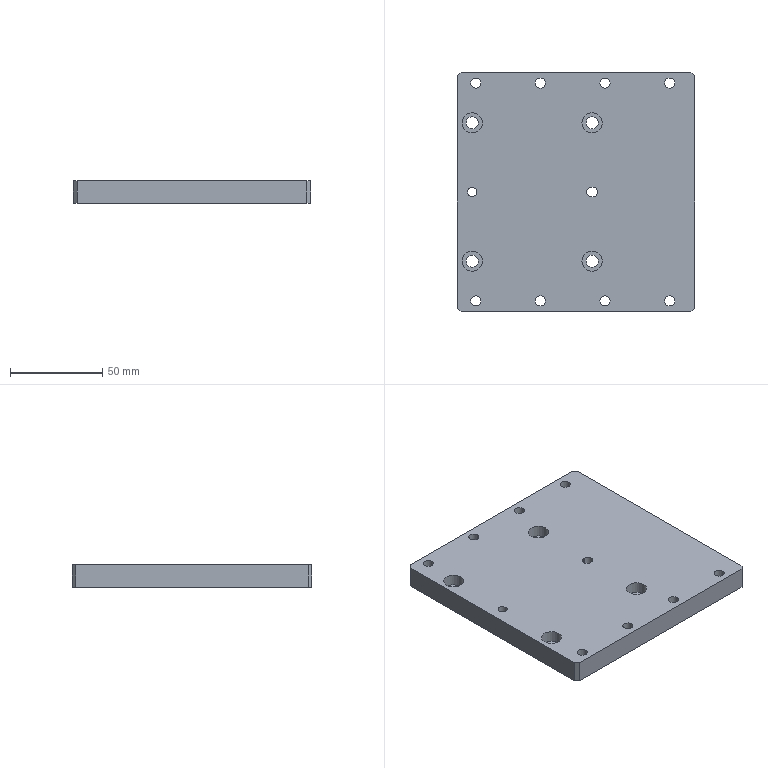Part | 1 solid | 63 faces | box 128.5 x 130 x 12 mm | volume 191153 mm3 | cylinder 33 | plane 24 | cone 6 | commonest cylinder face diameters 5.5 x8 10 x8 5 x5 4.2 x4 6.6 x4 11 x4
STEP:
#1=CARTESIAN_POINT('',(8.25,2.5,6.));
#2=VERTEX_POINT('',#1);
#3=CARTESIAN_POINT('',(8.25,-2.5,6.));
#4=VERTEX_POINT('',#3);
#5=CARTESIAN_POINT('',(8.25,0.,6.));
#6=DIRECTION('',(0.,0.,1.));
#7=DIRECTION('',(1.,0.,0.));
#8=AXIS2_PLACEMENT_3D('',#5,#6,#7);
#9=CIRCLE('',#8,2.5);
#10=EDGE_CURVE('',#2,#4,#9,.T.);
#11=ORIENTED_EDGE('',*,*,#10,.T.);
#12=CARTESIAN_POINT('',(8.25,-2.5,-6.));
#13=VERTEX_POINT('',#12);
#14=CARTESIAN_POINT('',(8.25,-2.5,6.));
#15=DIRECTION('',(0.,0.,1.));
#16=VECTOR('',#15,1000.);
#17=LINE('',#14,#16);
#18=EDGE_CURVE('',#13,#4,#17,.T.);
#19=ORIENTED_EDGE('',*,*,#18,.F.);
#20=CARTESIAN_POINT('',(8.25,2.5,-6.));
#21=VERTEX_POINT('',#20);
#22=CARTESIAN_POINT('',(8.25,0.,-6.));
#23=DIRECTION('',(0.,0.,1.));
#24=DIRECTION('',(1.,0.,0.));
#25=AXIS2_PLACEMENT_3D('',#22,#23,#24);
#26=CIRCLE('',#25,2.5);
#27=EDGE_CURVE('',#21,#13,#26,.T.);
#28=ORIENTED_EDGE('',*,*,#27,.F.);
#29=CARTESIAN_POINT('',(8.25,2.5,6.));
#30=DIRECTION('',(0.,0.,-1.));
#31=VECTOR('',#30,1000.);
#32=LINE('',#29,#31);
#33=EDGE_CURVE('',#2,#21,#32,.T.);
#34=ORIENTED_EDGE('',*,*,#33,.F.);
#35=EDGE_LOOP('',(#11,#19,#28,#34));
#36=FACE_BOUND('',#35,.T.);
#37=CARTESIAN_POINT('',(8.25,0.,6.));
#38=DIRECTION('',(0.,0.,1.));
#39=DIRECTION('',(1.,0.,0.));
#40=AXIS2_PLACEMENT_3D('',#37,#38,#39);
#41=CYLINDRICAL_SURFACE('',#40,2.5);
#42=ADVANCED_FACE('',(#36),#41,.F.);
#43=CARTESIAN_POINT('',(9.25,2.5,6.));
#44=VERTEX_POINT('',#43);
#45=CARTESIAN_POINT('',(8.25,2.5,6.));
#46=DIRECTION('',(1.,0.,0.));
#47=VECTOR('',#46,1000.);
#48=LINE('',#45,#47);
#49=EDGE_CURVE('',#2,#44,#48,.T.);
#50=ORIENTED_EDGE('',*,*,#49,.F.);
#51=ORIENTED_EDGE('',*,*,#33,.T.);
#52=CARTESIAN_POINT('',(9.25,2.5,-6.));
#53=VERTEX_POINT('',#52);
#54=CARTESIAN_POINT('',(8.25,2.5,-6.));
#55=DIRECTION('',(1.,0.,0.));
#56=VECTOR('',#55,1000.);
#57=LINE('',#54,#56);
#58=EDGE_CURVE('',#21,#53,#57,.T.);
#59=ORIENTED_EDGE('',*,*,#58,.T.);
#60=CARTESIAN_POINT('',(9.25,2.5,6.));
#61=DIRECTION('',(0.,0.,1.));
#62=VECTOR('',#61,1000.);
#63=LINE('',#60,#62);
#64=EDGE_CURVE('',#53,#44,#63,.T.);
#65=ORIENTED_EDGE('',*,*,#64,.T.);
#66=EDGE_LOOP('',(#50,#51,#59,#65));
#67=FACE_BOUND('',#66,.T.);
#68=CARTESIAN_POINT('',(8.25,2.5,6.));
#69=DIRECTION('',(0.,1.,0.));
#70=DIRECTION('',(-1.,0.,0.));
#71=AXIS2_PLACEMENT_3D('',#68,#69,#70);
#72=PLANE('',#71);
#73=ADVANCED_FACE('',(#67),#72,.F.);
#74=CARTESIAN_POINT('',(9.25,-2.5,6.));
#75=VERTEX_POINT('',#74);
#76=CARTESIAN_POINT('',(8.25,-2.5,6.));
#77=DIRECTION('',(1.,0.,0.));
#78=VECTOR('',#77,1000.);
#79=LINE('',#76,#78);
#80=EDGE_CURVE('',#4,#75,#79,.T.);
#81=ORIENTED_EDGE('',*,*,#80,.T.);
#82=CARTESIAN_POINT('',(9.25,-2.5,-6.));
#83=VERTEX_POINT('',#82);
#84=CARTESIAN_POINT('',(9.25,-2.5,6.));
#85=DIRECTION('',(0.,0.,-1.));
#86=VECTOR('',#85,1000.);
#87=LINE('',#84,#86);
#88=EDGE_CURVE('',#75,#83,#87,.T.);
#89=ORIENTED_EDGE('',*,*,#88,.T.);
#90=CARTESIAN_POINT('',(0.,-2.5,-6.));
#91=DIRECTION('',(1.,0.,0.));
#92=VECTOR('',#91,1000.);
#93=LINE('',#90,#92);
#94=EDGE_CURVE('',#13,#83,#93,.T.);
#95=ORIENTED_EDGE('',*,*,#94,.F.);
#96=ORIENTED_EDGE('',*,*,#18,.T.);
#97=EDGE_LOOP('',(#81,#89,#95,#96));
#98=FACE_BOUND('',#97,.T.);
#99=CARTESIAN_POINT('',(8.25,-2.5,6.));
#100=DIRECTION('',(0.,-1.,0.));
#101=DIRECTION('',(1.,0.,0.));
#102=AXIS2_PLACEMENT_3D('',#99,#100,#101);
#103=PLANE('',#102);
#104=ADVANCED_FACE('',(#98),#103,.F.);
#105=CARTESIAN_POINT('',(64.25,63.,6.));
#106=VERTEX_POINT('',#105);
#107=CARTESIAN_POINT('',(62.25,65.,6.));
#108=VERTEX_POINT('',#107);
#109=CARTESIAN_POINT('',(63.625,63.625,6.));
#110=DIRECTION('',(-0.7071,0.7071,0.));
#111=VECTOR('',#110,1000.);
#112=LINE('',#109,#111);
#113=EDGE_CURVE('',#106,#108,#112,.T.);
#114=ORIENTED_EDGE('',*,*,#113,.F.);
#115=CARTESIAN_POINT('',(64.25,63.,-6.));
#116=VERTEX_POINT('',#115);
#117=CARTESIAN_POINT('',(64.25,63.,6.));
#118=DIRECTION('',(0.,0.,1.));
#119=VECTOR('',#118,1000.);
#120=LINE('',#117,#119);
#121=EDGE_CURVE('',#116,#106,#120,.T.);
#122=ORIENTED_EDGE('',*,*,#121,.F.);
#123=CARTESIAN_POINT('',(62.25,65.,-6.));
#124=VERTEX_POINT('',#123);
#125=CARTESIAN_POINT('',(62.25,65.,-6.));
#126=DIRECTION('',(0.7071,-0.7071,0.));
#127=VECTOR('',#126,1000.);
#128=LINE('',#125,#127);
#129=EDGE_CURVE('',#124,#116,#128,.T.);
#130=ORIENTED_EDGE('',*,*,#129,.F.);
#131=CARTESIAN_POINT('',(62.25,65.,6.));
#132=DIRECTION('',(0.,0.,-1.));
#133=VECTOR('',#132,1000.);
#134=LINE('',#131,#133);
#135=EDGE_CURVE('',#108,#124,#134,.T.);
#136=ORIENTED_EDGE('',*,*,#135,.F.);
#137=EDGE_LOOP('',(#114,#122,#130,#136));
#138=FACE_BOUND('',#137,.T.);
#139=CARTESIAN_POINT('',(62.25,65.,6.));
#140=DIRECTION('',(-0.7071,-0.7071,0.));
#141=DIRECTION('',(0.,0.,-1.));
#142=AXIS2_PLACEMENT_3D('',#139,#140,#141);
#143=PLANE('',#142);
#144=ADVANCED_FACE('',(#138),#143,.F.);
#145=CARTESIAN_POINT('',(62.25,-65.,6.));
#146=VERTEX_POINT('',#145);
#147=CARTESIAN_POINT('',(64.25,-63.,6.));
#148=VERTEX_POINT('',#147);
#149=CARTESIAN_POINT('',(63.625,-63.625,6.));
#150=DIRECTION('',(0.7071,0.7071,0.));
#151=VECTOR('',#150,1000.);
#152=LINE('',#149,#151);
#153=EDGE_CURVE('',#146,#148,#152,.T.);
#154=ORIENTED_EDGE('',*,*,#153,.F.);
#155=CARTESIAN_POINT('',(62.25,-65.,-6.));
#156=VERTEX_POINT('',#155);
#157=CARTESIAN_POINT('',(62.25,-65.,6.));
#158=DIRECTION('',(0.,0.,1.));
#159=VECTOR('',#158,1000.);
#160=LINE('',#157,#159);
#161=EDGE_CURVE('',#156,#146,#160,.T.);
#162=ORIENTED_EDGE('',*,*,#161,.F.);
#163=CARTESIAN_POINT('',(64.25,-63.,-6.));
#164=VERTEX_POINT('',#163);
#165=CARTESIAN_POINT('',(64.25,-63.,-6.));
#166=DIRECTION('',(-0.7071,-0.7071,0.));
#167=VECTOR('',#166,1000.);
#168=LINE('',#165,#167);
#169=EDGE_CURVE('',#164,#156,#168,.T.);
#170=ORIENTED_EDGE('',*,*,#169,.F.);
#171=CARTESIAN_POINT('',(64.25,-63.,6.));
#172=DIRECTION('',(0.,0.,-1.));
#173=VECTOR('',#172,1000.);
#174=LINE('',#171,#173);
#175=EDGE_CURVE('',#148,#164,#174,.T.);
#176=ORIENTED_EDGE('',*,*,#175,.F.);
#177=EDGE_LOOP('',(#154,#162,#170,#176));
#178=FACE_BOUND('',#177,.T.);
#179=CARTESIAN_POINT('',(64.25,-63.,6.));
#180=DIRECTION('',(-0.7071,0.7071,0.));
#181=DIRECTION('',(0.,0.,-1.));
#182=AXIS2_PLACEMENT_3D('',#179,#180,#181);
#183=PLANE('',#182);
#184=ADVANCED_FACE('',(#178),#183,.F.);
#185=CARTESIAN_POINT('',(-64.25,-63.,6.));
#186=VERTEX_POINT('',#185);
#187=CARTESIAN_POINT('',(-62.25,-65.,6.));
#188=VERTEX_POINT('',#187);
#189=CARTESIAN_POINT('',(-63.625,-63.625,6.));
#190=DIRECTION('',(0.7071,-0.7071,0.));
#191=VECTOR('',#190,1000.);
#192=LINE('',#189,#191);
#193=EDGE_CURVE('',#186,#188,#192,.T.);
#194=ORIENTED_EDGE('',*,*,#193,.F.);
#195=CARTESIAN_POINT('',(-64.25,-63.,-6.));
#196=VERTEX_POINT('',#195);
#197=CARTESIAN_POINT('',(-64.25,-63.,6.));
#198=DIRECTION('',(0.,0.,1.));
#199=VECTOR('',#198,1000.);
#200=LINE('',#197,#199);
#201=EDGE_CURVE('',#196,#186,#200,.T.);
#202=ORIENTED_EDGE('',*,*,#201,.F.);
#203=CARTESIAN_POINT('',(-62.25,-65.,-6.));
#204=VERTEX_POINT('',#203);
#205=CARTESIAN_POINT('',(-62.25,-65.,-6.));
#206=DIRECTION('',(-0.7071,0.7071,0.));
#207=VECTOR('',#206,1000.);
#208=LINE('',#205,#207);
#209=EDGE_CURVE('',#204,#196,#208,.T.);
#210=ORIENTED_EDGE('',*,*,#209,.F.);
#211=CARTESIAN_POINT('',(-62.25,-65.,6.));
#212=DIRECTION('',(0.,0.,-1.));
#213=VECTOR('',#212,1000.);
#214=LINE('',#211,#213);
#215=EDGE_CURVE('',#188,#204,#214,.T.);
#216=ORIENTED_EDGE('',*,*,#215,.F.);
#217=EDGE_LOOP('',(#194,#202,#210,#216));
#218=FACE_BOUND('',#217,.T.);
#219=CARTESIAN_POINT('',(-62.25,-65.,6.));
#220=DIRECTION('',(0.7071,0.7071,0.));
#221=DIRECTION('',(0.,0.,-1.));
#222=AXIS2_PLACEMENT_3D('',#219,#220,#221);
#223=PLANE('',#222);
#224=ADVANCED_FACE('',(#218),#223,.F.);
#225=CARTESIAN_POINT('',(-62.25,65.,6.));
#226=VERTEX_POINT('',#225);
#227=CARTESIAN_POINT('',(-64.25,63.,6.));
#228=VERTEX_POINT('',#227);
#229=CARTESIAN_POINT('',(-63.625,63.625,6.));
#230=DIRECTION('',(-0.7071,-0.7071,0.));
#231=VECTOR('',#230,1000.);
#232=LINE('',#229,#231);
#233=EDGE_CURVE('',#226,#228,#232,.T.);
#234=ORIENTED_EDGE('',*,*,#233,.F.);
#235=CARTESIAN_POINT('',(-62.25,65.,-6.));
#236=VERTEX_POINT('',#235);
#237=CARTESIAN_POINT('',(-62.25,65.,6.));
#238=DIRECTION('',(0.,0.,1.));
#239=VECTOR('',#238,1000.);
#240=LINE('',#237,#239);
#241=EDGE_CURVE('',#236,#226,#240,.T.);
#242=ORIENTED_EDGE('',*,*,#241,.F.);
#243=CARTESIAN_POINT('',(-64.25,63.,-6.));
#244=VERTEX_POINT('',#243);
#245=CARTESIAN_POINT('',(-64.25,63.,-6.));
#246=DIRECTION('',(0.7071,0.7071,0.));
#247=VECTOR('',#246,1000.);
#248=LINE('',#245,#247);
#249=EDGE_CURVE('',#244,#236,#248,.T.);
#250=ORIENTED_EDGE('',*,*,#249,.F.);
#251=CARTESIAN_POINT('',(-64.25,63.,6.));
#252=DIRECTION('',(0.,0.,-1.));
#253=VECTOR('',#252,1000.);
#254=LINE('',#251,#253);
#255=EDGE_CURVE('',#228,#244,#254,.T.);
#256=ORIENTED_EDGE('',*,*,#255,.F.);
#257=EDGE_LOOP('',(#234,#242,#250,#256));
#258=FACE_BOUND('',#257,.T.);
#259=CARTESIAN_POINT('',(-64.25,63.,6.));
#260=DIRECTION('',(0.7071,-0.7071,0.));
#261=DIRECTION('',(0.,0.,-1.));
#262=AXIS2_PLACEMENT_3D('',#259,#260,#261);
#263=PLANE('',#262);
#264=ADVANCED_FACE('',(#258),#263,.F.);
#265=CARTESIAN_POINT('',(-49.25,-59.,-0.6));
#266=VERTEX_POINT('',#265);
#267=CARTESIAN_POINT('',(-54.25,-59.,-0.6));
#268=DIRECTION('',(0.,0.,-1.));
#269=DIRECTION('',(1.,0.,0.));
#270=AXIS2_PLACEMENT_3D('',#267,#268,#269);
#271=CIRCLE('',#270,5.);
#272=EDGE_CURVE('',#266,#266,#271,.T.);
#273=ORIENTED_EDGE('',*,*,#272,.T.);
#274=EDGE_LOOP('',(#273));
#275=FACE_BOUND('',#274,.T.);
#276=CARTESIAN_POINT('',(-51.5,-59.,-0.6));
#277=VERTEX_POINT('',#276);
#278=CARTESIAN_POINT('',(-54.25,-59.,-0.6));
#279=DIRECTION('',(0.,0.,-1.));
#280=DIRECTION('',(1.,0.,0.));
#281=AXIS2_PLACEMENT_3D('',#278,#279,#280);
#282=CIRCLE('',#281,2.75);
#283=EDGE_CURVE('',#277,#277,#282,.T.);
#284=ORIENTED_EDGE('',*,*,#283,.F.);
#285=EDGE_LOOP('',(#284));
#286=FACE_BOUND('',#285,.T.);
#287=CARTESIAN_POINT('',(53.5,59.,-0.6));
#288=DIRECTION('',(0.,0.,1.));
#289=DIRECTION('',(1.,0.,0.));
#290=AXIS2_PLACEMENT_3D('',#287,#288,#289);
#291=PLANE('',#290);
#292=ADVANCED_FACE('',(#275,#286),#291,.F.);
#293=CARTESIAN_POINT('',(-14.25,-59.,-0.6));
#294=VERTEX_POINT('',#293);
#295=CARTESIAN_POINT('',(-19.25,-59.,-0.6));
#296=DIRECTION('',(0.,0.,-1.));
#297=DIRECTION('',(1.,0.,0.));
#298=AXIS2_PLACEMENT_3D('',#295,#296,#297);
#299=CIRCLE('',#298,5.);
#300=EDGE_CURVE('',#294,#294,#299,.T.);
#301=ORIENTED_EDGE('',*,*,#300,.T.);
#302=EDGE_LOOP('',(#301));
#303=FACE_BOUND('',#302,.T.);
#304=CARTESIAN_POINT('',(-16.5,-59.,-0.6));
#305=VERTEX_POINT('',#304);
#306=CARTESIAN_POINT('',(-19.25,-59.,-0.6));
#307=DIRECTION('',(0.,0.,-1.));
#308=DIRECTION('',(1.,0.,0.));
#309=AXIS2_PLACEMENT_3D('',#306,#307,#308);
#310=CIRCLE('',#309,2.75);
#311=EDGE_CURVE('',#305,#305,#310,.T.);
#312=ORIENTED_EDGE('',*,*,#311,.F.);
#313=EDGE_LOOP('',(#312));
#314=FACE_BOUND('',#313,.T.);
#315=CARTESIAN_POINT('',(53.5,59.,-0.6));
#316=DIRECTION('',(0.,0.,1.));
#317=DIRECTION('',(1.,0.,0.));
#318=AXIS2_PLACEMENT_3D('',#315,#316,#317);
#319=PLANE('',#318);
#320=ADVANCED_FACE('',(#303,#314),#319,.F.);
#321=CARTESIAN_POINT('',(20.75,-59.,-0.6));
#322=VERTEX_POINT('',#321);
#323=CARTESIAN_POINT('',(15.75,-59.,-0.6));
#324=DIRECTION('',(0.,0.,-1.));
#325=DIRECTION('',(1.,0.,0.));
#326=AXIS2_PLACEMENT_3D('',#323,#324,#325);
#327=CIRCLE('',#326,5.);
#328=EDGE_CURVE('',#322,#322,#327,.T.);
#329=ORIENTED_EDGE('',*,*,#328,.T.);
#330=EDGE_LOOP('',(#329));
#331=FACE_BOUND('',#330,.T.);
#332=CARTESIAN_POINT('',(18.5,-59.,-0.6));
#333=VERTEX_POINT('',#332);
#334=CARTESIAN_POINT('',(15.75,-59.,-0.6));
#335=DIRECTION('',(0.,0.,-1.));
#336=DIRECTION('',(1.,0.,0.));
#337=AXIS2_PLACEMENT_3D('',#334,#335,#336);
#338=CIRCLE('',#337,2.75);
#339=EDGE_CURVE('',#333,#333,#338,.T.);
#340=ORIENTED_EDGE('',*,*,#339,.F.);
#341=EDGE_LOOP('',(#340));
#342=FACE_BOUND('',#341,.T.);
#343=CARTESIAN_POINT('',(53.5,59.,-0.6));
#344=DIRECTION('',(0.,0.,1.));
#345=DIRECTION('',(1.,0.,0.));
#346=AXIS2_PLACEMENT_3D('',#343,#344,#345);
#347=PLANE('',#346);
#348=ADVANCED_FACE('',(#331,#342),#347,.F.);
#349=CARTESIAN_POINT('',(-49.25,59.,-0.6));
#350=VERTEX_POINT('',#349);
#351=CARTESIAN_POINT('',(-54.25,59.,-0.6));
#352=DIRECTION('',(0.,0.,-1.));
#353=DIRECTION('',(1.,0.,0.));
#354=AXIS2_PLACEMENT_3D('',#351,#352,#353);
#355=CIRCLE('',#354,5.);
#356=EDGE_CURVE('',#350,#350,#355,.T.);
#357=ORIENTED_EDGE('',*,*,#356,.T.);
#358=EDGE_LOOP('',(#357));
#359=FACE_BOUND('',#358,.T.);
#360=CARTESIAN_POINT('',(-51.5,59.,-0.6));
#361=VERTEX_POINT('',#360);
#362=CARTESIAN_POINT('',(-54.25,59.,-0.6));
#363=DIRECTION('',(0.,0.,-1.));
#364=DIRECTION('',(1.,0.,0.));
#365=AXIS2_PLACEMENT_3D('',#362,#363,#364);
#366=CIRCLE('',#365,2.75);
#367=EDGE_CURVE('',#361,#361,#366,.T.);
#368=ORIENTED_EDGE('',*,*,#367,.F.);
#369=EDGE_LOOP('',(#368));
#370=FACE_BOUND('',#369,.T.);
#371=CARTESIAN_POINT('',(53.5,59.,-0.6));
#372=DIRECTION('',(0.,0.,1.));
#373=DIRECTION('',(1.,0.,0.));
#374=AXIS2_PLACEMENT_3D('',#371,#372,#373);
#375=PLANE('',#374);
#376=ADVANCED_FACE('',(#359,#370),#375,.F.);
#377=CARTESIAN_POINT('',(-14.25,59.,-0.6));
#378=VERTEX_POINT('',#377);
#379=CARTESIAN_POINT('',(-19.25,59.,-0.6));
#380=DIRECTION('',(0.,0.,-1.));
#381=DIRECTION('',(1.,0.,0.));
#382=AXIS2_PLACEMENT_3D('',#379,#380,#381);
#383=CIRCLE('',#382,5.);
#384=EDGE_CURVE('',#378,#378,#383,.T.);
#385=ORIENTED_EDGE('',*,*,#384,.T.);
#386=EDGE_LOOP('',(#385));
#387=FACE_BOUND('',#386,.T.);
#388=CARTESIAN_POINT('',(-16.5,59.,-0.6));
#389=VERTEX_POINT('',#388);
#390=CARTESIAN_POINT('',(-19.25,59.,-0.6));
#391=DIRECTION('',(0.,0.,-1.));
#392=DIRECTION('',(1.,0.,0.));
#393=AXIS2_PLACEMENT_3D('',#390,#391,#392);
#394=CIRCLE('',#393,2.75);
#395=EDGE_CURVE('',#389,#389,#394,.T.);
#396=ORIENTED_EDGE('',*,*,#395,.F.);
#397=EDGE_LOOP('',(#396));
#398=FACE_BOUND('',#397,.T.);
#399=CARTESIAN_POINT('',(53.5,59.,-0.6));
#400=DIRECTION('',(0.,0.,1.));
#401=DIRECTION('',(1.,0.,0.));
#402=AXIS2_PLACEMENT_3D('',#399,#400,#401);
#403=PLANE('',#402);
#404=ADVANCED_FACE('',(#387,#398),#403,.F.);
#405=CARTESIAN_POINT('',(20.75,59.,-0.6));
#406=VERTEX_POINT('',#405);
#407=CARTESIAN_POINT('',(15.75,59.,-0.6));
#408=DIRECTION('',(0.,0.,-1.));
#409=DIRECTION('',(1.,0.,0.));
#410=AXIS2_PLACEMENT_3D('',#407,#408,#409);
#411=CIRCLE('',#410,5.);
#412=EDGE_CURVE('',#406,#406,#411,.T.);
#413=ORIENTED_EDGE('',*,*,#412,.T.);
#414=EDGE_LOOP('',(#413));
#415=FACE_BOUND('',#414,.T.);
#416=CARTESIAN_POINT('',(18.5,59.,-0.6));
#417=VERTEX_POINT('',#416);
#418=CARTESIAN_POINT('',(15.75,59.,-0.6));
#419=DIRECTION('',(0.,0.,-1.));
#420=DIRECTION('',(1.,0.,0.));
#421=AXIS2_PLACEMENT_3D('',#418,#419,#420);
#422=CIRCLE('',#421,2.75);
#423=EDGE_CURVE('',#417,#417,#422,.T.);
#424=ORIENTED_EDGE('',*,*,#423,.F.);
#425=EDGE_LOOP('',(#424));
#426=FACE_BOUND('',#425,.T.);
#427=CARTESIAN_POINT('',(53.5,59.,-0.6));
#428=DIRECTION('',(0.,0.,1.));
#429=DIRECTION('',(1.,0.,0.));
#430=AXIS2_PLACEMENT_3D('',#427,#428,#429);
#431=PLANE('',#430);
#432=ADVANCED_FACE('',(#415,#426),#431,.F.);
#433=CARTESIAN_POINT('',(55.75,-59.,-0.6));
#434=VERTEX_POINT('',#433);
#435=CARTESIAN_POINT('',(50.75,-59.,-0.6));
#436=DIRECTION('',(0.,0.,-1.));
#437=DIRECTION('',(1.,0.,0.));
#438=AXIS2_PLACEMENT_3D('',#435,#436,#437);
#439=CIRCLE('',#438,5.);
#440=EDGE_CURVE('',#434,#434,#439,.T.);
#441=ORIENTED_EDGE('',*,*,#440,.T.);
#442=EDGE_LOOP('',(#441));
#443=FACE_BOUND('',#442,.T.);
#444=CARTESIAN_POINT('',(53.5,-59.,-0.6));
#445=VERTEX_POINT('',#444);
#446=CARTESIAN_POINT('',(50.75,-59.,-0.6));
#447=DIRECTION('',(0.,0.,-1.));
#448=DIRECTION('',(1.,0.,0.));
#449=AXIS2_PLACEMENT_3D('',#446,#447,#448);
#450=CIRCLE('',#449,2.75);
#451=EDGE_CURVE('',#445,#445,#450,.T.);
#452=ORIENTED_EDGE('',*,*,#451,.F.);
#453=EDGE_LOOP('',(#452));
#454=FACE_BOUND('',#453,.T.);
#455=CARTESIAN_POINT('',(53.5,59.,-0.6));
#456=DIRECTION('',(0.,0.,1.));
#457=DIRECTION('',(1.,0.,0.));
#458=AXIS2_PLACEMENT_3D('',#455,#456,#457);
#459=PLANE('',#458);
#460=ADVANCED_FACE('',(#443,#454),#459,.F.);
#461=CARTESIAN_POINT('',(45.75,59.,-0.6));
#462=VERTEX_POINT('',#461);
#463=CARTESIAN_POINT('',(50.75,59.,-0.6));
#464=DIRECTION('',(0.,0.,-1.));
#465=DIRECTION('',(-1.,0.,0.));
#466=AXIS2_PLACEMENT_3D('',#463,#464,#465);
#467=CIRCLE('',#466,5.);
#468=EDGE_CURVE('',#462,#462,#467,.T.);
#469=ORIENTED_EDGE('',*,*,#468,.T.);
#470=EDGE_LOOP('',(#469));
#471=FACE_BOUND('',#470,.T.);
#472=CARTESIAN_POINT('',(48.,59.,-0.6));
#473=VERTEX_POINT('',#472);
#474=CARTESIAN_POINT('',(50.75,59.,-0.6));
#475=DIRECTION('',(0.,0.,-1.));
#476=DIRECTION('',(-1.,0.,0.));
#477=AXIS2_PLACEMENT_3D('',#474,#475,#476);
#478=CIRCLE('',#477,2.75);
#479=EDGE_CURVE('',#473,#473,#478,.T.);
#480=ORIENTED_EDGE('',*,*,#479,.F.);
#481=EDGE_LOOP('',(#480));
#482=FACE_BOUND('',#481,.T.);
#483=CARTESIAN_POINT('',(53.5,59.,-0.6));
#484=DIRECTION('',(0.,0.,1.));
#485=DIRECTION('',(1.,0.,0.));
#486=AXIS2_PLACEMENT_3D('',#483,#484,#485);
#487=PLANE('',#486);
#488=ADVANCED_FACE('',(#471,#482),#487,.F.);
#489=CARTESIAN_POINT('',(-61.75,-37.5,-0.4));
#490=VERTEX_POINT('',#489);
#491=CARTESIAN_POINT('',(-56.25,-37.5,-0.4));
#492=DIRECTION('',(0.,0.,1.));
#493=DIRECTION('',(-1.,0.,0.));
#494=AXIS2_PLACEMENT_3D('',#491,#492,#493);
#495=CIRCLE('',#494,5.5);
#496=EDGE_CURVE('',#490,#490,#495,.T.);
#497=ORIENTED_EDGE('',*,*,#496,.T.);
#498=EDGE_LOOP('',(#497));
#499=FACE_BOUND('',#498,.T.);
#500=CARTESIAN_POINT('',(-59.55,-37.5,-0.4));
#501=VERTEX_POINT('',#500);
#502=CARTESIAN_POINT('',(-56.25,-37.5,-0.4));
#503=DIRECTION('',(0.,0.,1.));
#504=DIRECTION('',(-1.,0.,0.));
#505=AXIS2_PLACEMENT_3D('',#502,#503,#504);
#506=CIRCLE('',#505,3.3);
#507=EDGE_CURVE('',#501,#501,#506,.T.);
#508=ORIENTED_EDGE('',*,*,#507,.F.);
#509=EDGE_LOOP('',(#508));
#510=FACE_BOUND('',#509,.T.);
#511=CARTESIAN_POINT('',(12.05,-37.5,-0.4));
#512=DIRECTION('',(0.,0.,-1.));
#513=DIRECTION('',(-1.,0.,0.));
#514=AXIS2_PLACEMENT_3D('',#511,#512,#513);
#515=PLANE('',#514);
#516=ADVANCED_FACE('',(#499,#510),#515,.F.);
#517=CARTESIAN_POINT('',(-61.75,37.5,-0.4));
#518=VERTEX_POINT('',#517);
#519=CARTESIAN_POINT('',(-56.25,37.5,-0.4));
#520=DIRECTION('',(0.,0.,1.));
#521=DIRECTION('',(-1.,0.,0.));
#522=AXIS2_PLACEMENT_3D('',#519,#520,#521);
#523=CIRCLE('',#522,5.5);
#524=EDGE_CURVE('',#518,#518,#523,.T.);
#525=ORIENTED_EDGE('',*,*,#524,.T.);
#526=EDGE_LOOP('',(#525));
#527=FACE_BOUND('',#526,.T.);
#528=CARTESIAN_POINT('',(-59.55,37.5,-0.4));
#529=VERTEX_POINT('',#528);
#530=CARTESIAN_POINT('',(-56.25,37.5,-0.4));
#531=DIRECTION('',(0.,0.,1.));
#532=DIRECTION('',(-1.,0.,0.));
#533=AXIS2_PLACEMENT_3D('',#530,#531,#532);
#534=CIRCLE('',#533,3.3);
#535=EDGE_CURVE('',#529,#529,#534,.T.);
#536=ORIENTED_EDGE('',*,*,#535,.F.);
#537=EDGE_LOOP('',(#536));
#538=FACE_BOUND('',#537,.T.);
#539=CARTESIAN_POINT('',(12.05,-37.5,-0.4));
#540=DIRECTION('',(0.,0.,-1.));
#541=DIRECTION('',(-1.,0.,0.));
#542=AXIS2_PLACEMENT_3D('',#539,#540,#541);
#543=PLANE('',#542);
#544=ADVANCED_FACE('',(#527,#538),#543,.F.);
#545=CARTESIAN_POINT('',(3.25,37.5,-0.4));
#546=VERTEX_POINT('',#545);
#547=CARTESIAN_POINT('',(8.75,37.5,-0.4));
#548=DIRECTION('',(0.,0.,1.));
#549=DIRECTION('',(-1.,0.,0.));
#550=AXIS2_PLACEMENT_3D('',#547,#548,#549);
#551=CIRCLE('',#550,5.5);
#552=EDGE_CURVE('',#546,#546,#551,.T.);
#553=ORIENTED_EDGE('',*,*,#552,.T.);
#554=EDGE_LOOP('',(#553));
#555=FACE_BOUND('',#554,.T.);
#556=CARTESIAN_POINT('',(5.45,37.5,-0.4));
#557=VERTEX_POINT('',#556);
#558=CARTESIAN_POINT('',(8.75,37.5,-0.4));
#559=DIRECTION('',(0.,0.,1.));
#560=DIRECTION('',(-1.,0.,0.));
#561=AXIS2_PLACEMENT_3D('',#558,#559,#560);
#562=CIRCLE('',#561,3.3);
#563=EDGE_CURVE('',#557,#557,#562,.T.);
#564=ORIENTED_EDGE('',*,*,#563,.F.);
#565=EDGE_LOOP('',(#564));
#566=FACE_BOUND('',#565,.T.);
#567=CARTESIAN_POINT('',(12.05,-37.5,-0.4));
#568=DIRECTION('',(0.,0.,-1.));
#569=DIRECTION('',(-1.,0.,0.));
#570=AXIS2_PLACEMENT_3D('',#567,#568,#569);
#571=PLANE('',#570);
#572=ADVANCED_FACE('',(#555,#566),#571,.F.);
#573=CARTESIAN_POINT('',(14.25,-37.5,-0.4));
#574=VERTEX_POINT('',#573);
#575=CARTESIAN_POINT('',(8.75,-37.5,-0.4));
#576=DIRECTION('',(0.,0.,1.));
#577=DIRECTION('',(1.,0.,0.));
#578=AXIS2_PLACEMENT_3D('',#575,#576,#577);
#579=CIRCLE('',#578,5.5);
#580=EDGE_CURVE('',#574,#574,#579,.T.);
#581=ORIENTED_EDGE('',*,*,#580,.T.);
#582=EDGE_LOOP('',(#581));
#583=FACE_BOUND('',#582,.T.);
#584=CARTESIAN_POINT('',(12.05,-37.5,-0.4));
#585=VERTEX_POINT('',#584);
#586=CARTESIAN_POINT('',(8.75,-37.5,-0.4));
#587=DIRECTION('',(0.,0.,1.));
#588=DIRECTION('',(1.,0.,0.));
#589=AXIS2_PLACEMENT_3D('',#586,#587,#588);
#590=CIRCLE('',#589,3.3);
#591=EDGE_CURVE('',#585,#585,#590,.T.);
#592=ORIENTED_EDGE('',*,*,#591,.F.);
#593=EDGE_LOOP('',(#592));
#594=FACE_BOUND('',#593,.T.);
#595=CARTESIAN_POINT('',(12.05,-37.5,-0.4));
#596=DIRECTION('',(0.,0.,-1.));
#597=DIRECTION('',(-1.,0.,0.));
#598=AXIS2_PLACEMENT_3D('',#595,#596,#597);
#599=PLANE('',#598);
#600=ADVANCED_FACE('',(#583,#594),#599,.F.);
#601=CARTESIAN_POINT('',(-64.25,65.,-6.));
#602=DIRECTION('',(0.,-1.,0.));
#603=VECTOR('',#602,1000.);
#604=LINE('',#601,#603);
#605=EDGE_CURVE('',#244,#196,#604,.T.);
#606=ORIENTED_EDGE('',*,*,#605,.F.);
#607=ORIENTED_EDGE('',*,*,#249,.T.);
#608=CARTESIAN_POINT('',(-64.25,65.,-6.));
#609=DIRECTION('',(-1.,0.,0.));
#610=VECTOR('',#609,1000.);
#611=LINE('',#608,#610);
#612=EDGE_CURVE('',#124,#236,#611,.T.);
#613=ORIENTED_EDGE('',*,*,#612,.F.);
#614=ORIENTED_EDGE('',*,*,#129,.T.);
#615=CARTESIAN_POINT('',(64.25,65.,-6.));
#616=DIRECTION('',(0.,1.,0.));
#617=VECTOR('',#616,1000.);
#618=LINE('',#615,#617);
#619=EDGE_CURVE('',#164,#116,#618,.T.);
#620=ORIENTED_EDGE('',*,*,#619,.F.);
#621=ORIENTED_EDGE('',*,*,#169,.T.);
#622=CARTESIAN_POINT('',(-64.25,-65.,-6.));
#623=DIRECTION('',(1.,0.,0.));
#624=VECTOR('',#623,1000.);
#625=LINE('',#622,#624);
#626=EDGE_CURVE('',#204,#156,#625,.T.);
#627=ORIENTED_EDGE('',*,*,#626,.F.);
#628=ORIENTED_EDGE('',*,*,#209,.T.);
#629=EDGE_LOOP('',(#606,#607,#613,#614,#620,#621,#627,#628));
#630=FACE_BOUND('',#629,.T.);
#631=CARTESIAN_POINT('',(12.05,-37.5,-6.));
#632=VERTEX_POINT('',#631);
#633=CARTESIAN_POINT('',(8.75,-37.5,-6.));
#634=DIRECTION('',(0.,0.,1.));
#635=DIRECTION('',(1.,0.,0.));
#636=AXIS2_PLACEMENT_3D('',#633,#634,#635);
#637=CIRCLE('',#636,3.3);
#638=EDGE_CURVE('',#632,#632,#637,.T.);
#639=ORIENTED_EDGE('',*,*,#638,.T.);
#640=EDGE_LOOP('',(#639));
#641=FACE_BOUND('',#640,.T.);
#642=CARTESIAN_POINT('',(12.05,37.5,-6.));
#643=VERTEX_POINT('',#642);
#644=CARTESIAN_POINT('',(8.75,37.5,-6.));
#645=DIRECTION('',(0.,0.,1.));
#646=DIRECTION('',(1.,0.,0.));
#647=AXIS2_PLACEMENT_3D('',#644,#645,#646);
#648=CIRCLE('',#647,3.3);
#649=EDGE_CURVE('',#643,#643,#648,.T.);
#650=ORIENTED_EDGE('',*,*,#649,.T.);
#651=EDGE_LOOP('',(#650));
#652=FACE_BOUND('',#651,.T.);
#653=CARTESIAN_POINT('',(-52.95,37.5,-6.));
#654=VERTEX_POINT('',#653);
#655=CARTESIAN_POINT('',(-56.25,37.5,-6.));
#656=DIRECTION('',(0.,0.,1.));
#657=DIRECTION('',(1.,0.,0.));
#658=AXIS2_PLACEMENT_3D('',#655,#656,#657);
#659=CIRCLE('',#658,3.3);
#660=EDGE_CURVE('',#654,#654,#659,.T.);
#661=ORIENTED_EDGE('',*,*,#660,.T.);
#662=EDGE_LOOP('',(#661));
#663=FACE_BOUND('',#662,.T.);
#664=CARTESIAN_POINT('',(-52.95,-37.5,-6.));
#665=VERTEX_POINT('',#664);
#666=CARTESIAN_POINT('',(-56.25,-37.5,-6.));
#667=DIRECTION('',(0.,0.,1.));
#668=DIRECTION('',(1.,0.,0.));
#669=AXIS2_PLACEMENT_3D('',#666,#667,#668);
#670=CIRCLE('',#669,3.3);
#671=EDGE_CURVE('',#665,#665,#670,.T.);
#672=ORIENTED_EDGE('',*,*,#671,.T.);
#673=EDGE_LOOP('',(#672));
#674=FACE_BOUND('',#673,.T.);
#675=CARTESIAN_POINT('',(45.75,59.,-6.));
#676=VERTEX_POINT('',#675);
#677=CARTESIAN_POINT('',(50.75,59.,-6.));
#678=DIRECTION('',(0.,0.,-1.));
#679=DIRECTION('',(-1.,0.,0.));
#680=AXIS2_PLACEMENT_3D('',#677,#678,#679);
#681=CIRCLE('',#680,5.);
#682=EDGE_CURVE('',#676,#676,#681,.T.);
#683=ORIENTED_EDGE('',*,*,#682,.F.);
#684=EDGE_LOOP('',(#683));
#685=FACE_BOUND('',#684,.T.);
#686=CARTESIAN_POINT('',(45.75,-59.,-6.));
#687=VERTEX_POINT('',#686);
#688=CARTESIAN_POINT('',(50.75,-59.,-6.));
#689=DIRECTION('',(0.,0.,-1.));
#690=DIRECTION('',(-1.,0.,0.));
#691=AXIS2_PLACEMENT_3D('',#688,#689,#690);
#692=CIRCLE('',#691,5.);
#693=EDGE_CURVE('',#687,#687,#692,.T.);
#694=ORIENTED_EDGE('',*,*,#693,.F.);
#695=EDGE_LOOP('',(#694));
#696=FACE_BOUND('',#695,.T.);
#697=CARTESIAN_POINT('',(10.75,59.,-6.));
#698=VERTEX_POINT('',#697);
#699=CARTESIAN_POINT('',(15.75,59.,-6.));
#700=DIRECTION('',(0.,0.,-1.));
#701=DIRECTION('',(-1.,0.,0.));
#702=AXIS2_PLACEMENT_3D('',#699,#700,#701);
#703=CIRCLE('',#702,5.);
#704=EDGE_CURVE('',#698,#698,#703,.T.);
#705=ORIENTED_EDGE('',*,*,#704,.F.);
#706=EDGE_LOOP('',(#705));
#707=FACE_BOUND('',#706,.T.);
#708=CARTESIAN_POINT('',(-24.25,59.,-6.));
#709=VERTEX_POINT('',#708);
#710=CARTESIAN_POINT('',(-19.25,59.,-6.));
#711=DIRECTION('',(0.,0.,-1.));
#712=DIRECTION('',(-1.,0.,0.));
#713=AXIS2_PLACEMENT_3D('',#710,#711,#712);
#714=CIRCLE('',#713,5.);
#715=EDGE_CURVE('',#709,#709,#714,.T.);
#716=ORIENTED_EDGE('',*,*,#715,.F.);
#717=EDGE_LOOP('',(#716));
#718=FACE_BOUND('',#717,.T.);
#719=CARTESIAN_POINT('',(-59.25,59.,-6.));
#720=VERTEX_POINT('',#719);
#721=CARTESIAN_POINT('',(-54.25,59.,-6.));
#722=DIRECTION('',(0.,0.,-1.));
#723=DIRECTION('',(-1.,0.,0.));
#724=AXIS2_PLACEMENT_3D('',#721,#722,#723);
#725=CIRCLE('',#724,5.);
#726=EDGE_CURVE('',#720,#720,#725,.T.);
#727=ORIENTED_EDGE('',*,*,#726,.F.);
#728=EDGE_LOOP('',(#727));
#729=FACE_BOUND('',#728,.T.);
#730=CARTESIAN_POINT('',(10.75,-59.,-6.));
#731=VERTEX_POINT('',#730);
#732=CARTESIAN_POINT('',(15.75,-59.,-6.));
#733=DIRECTION('',(0.,0.,-1.));
#734=DIRECTION('',(-1.,0.,0.));
#735=AXIS2_PLACEMENT_3D('',#732,#733,#734);
#736=CIRCLE('',#735,5.);
#737=EDGE_CURVE('',#731,#731,#736,.T.);
#738=ORIENTED_EDGE('',*,*,#737,.F.);
#739=EDGE_LOOP('',(#738));
#740=FACE_BOUND('',#739,.T.);
#741=CARTESIAN_POINT('',(-24.25,-59.,-6.));
#742=VERTEX_POINT('',#741);
#743=CARTESIAN_POINT('',(-19.25,-59.,-6.));
#744=DIRECTION('',(0.,0.,-1.));
#745=DIRECTION('',(-1.,0.,0.));
#746=AXIS2_PLACEMENT_3D('',#743,#744,#745);
#747=CIRCLE('',#746,5.);
#748=EDGE_CURVE('',#742,#742,#747,.T.);
#749=ORIENTED_EDGE('',*,*,#748,.F.);
#750=EDGE_LOOP('',(#749));
#751=FACE_BOUND('',#750,.T.);
#752=CARTESIAN_POINT('',(-59.25,-59.,-6.));
#753=VERTEX_POINT('',#752);
#754=CARTESIAN_POINT('',(-54.25,-59.,-6.));
#755=DIRECTION('',(0.,0.,-1.));
#756=DIRECTION('',(-1.,0.,0.));
#757=AXIS2_PLACEMENT_3D('',#754,#755,#756);
#758=CIRCLE('',#757,5.);
#759=EDGE_CURVE('',#753,#753,#758,.T.);
#760=ORIENTED_EDGE('',*,*,#759,.F.);
#761=EDGE_LOOP('',(#760));
#762=FACE_BOUND('',#761,.T.);
#763=ORIENTED_EDGE('',*,*,#27,.T.);
#764=ORIENTED_EDGE('',*,*,#94,.T.);
#765=CARTESIAN_POINT('',(9.25,0.,-6.));
#766=DIRECTION('',(0.,0.,1.));
#767=DIRECTION('',(1.,0.,0.));
#768=AXIS2_PLACEMENT_3D('',#765,#766,#767);
#769=CIRCLE('',#768,2.5);
#770=EDGE_CURVE('',#83,#53,#769,.T.);
#771=ORIENTED_EDGE('',*,*,#770,.T.);
#772=ORIENTED_EDGE('',*,*,#58,.F.);
#773=EDGE_LOOP('',(#763,#764,#771,#772));
#774=FACE_BOUND('',#773,.T.);
#775=CARTESIAN_POINT('',(-53.75,0.,-6.));
#776=VERTEX_POINT('',#775);
#777=CARTESIAN_POINT('',(-56.25,0.,-6.));
#778=DIRECTION('',(0.,0.,1.));
#779=DIRECTION('',(1.,0.,0.));
#780=AXIS2_PLACEMENT_3D('',#777,#778,#779);
#781=CIRCLE('',#780,2.5);
#782=EDGE_CURVE('',#776,#776,#781,.T.);
#783=ORIENTED_EDGE('',*,*,#782,.T.);
#784=EDGE_LOOP('',(#783));
#785=FACE_BOUND('',#784,.T.);
#786=CARTESIAN_POINT('',(0.,0.,-6.));
#787=DIRECTION('',(0.,0.,1.));
#788=DIRECTION('',(1.,0.,0.));
#789=AXIS2_PLACEMENT_3D('',#786,#787,#788);
#790=PLANE('',#789);
#791=ADVANCED_FACE('',(#630,#641,#652,#663,#674,#685,#696,#707,#718,#729,#740,#751,#762,#774,#785),#790,.F.);
#792=CARTESIAN_POINT('',(-64.25,65.,6.));
#793=DIRECTION('',(-1.,0.,0.));
#794=VECTOR('',#793,1000.);
#795=LINE('',#792,#794);
#796=EDGE_CURVE('',#108,#226,#795,.T.);
#797=ORIENTED_EDGE('',*,*,#796,.T.);
#798=ORIENTED_EDGE('',*,*,#233,.T.);
#799=CARTESIAN_POINT('',(-64.25,65.,6.));
#800=DIRECTION('',(0.,-1.,0.));
#801=VECTOR('',#800,1000.);
#802=LINE('',#799,#801);
#803=EDGE_CURVE('',#228,#186,#802,.T.);
#804=ORIENTED_EDGE('',*,*,#803,.T.);
#805=ORIENTED_EDGE('',*,*,#193,.T.);
#806=CARTESIAN_POINT('',(-64.25,-65.,6.));
#807=DIRECTION('',(1.,0.,0.));
#808=VECTOR('',#807,1000.);
#809=LINE('',#806,#808);
#810=EDGE_CURVE('',#188,#146,#809,.T.);
#811=ORIENTED_EDGE('',*,*,#810,.T.);
#812=ORIENTED_EDGE('',*,*,#153,.T.);
#813=CARTESIAN_POINT('',(64.25,65.,6.));
#814=DIRECTION('',(0.,1.,0.));
#815=VECTOR('',#814,1000.);
#816=LINE('',#813,#815);
#817=EDGE_CURVE('',#148,#106,#816,.T.);
#818=ORIENTED_EDGE('',*,*,#817,.T.);
#819=ORIENTED_EDGE('',*,*,#113,.T.);
#820=EDGE_LOOP('',(#797,#798,#804,#805,#811,#812,#818,#819));
#821=FACE_BOUND('',#820,.T.);
#822=CARTESIAN_POINT('',(14.25,-37.5,6.));
#823=VERTEX_POINT('',#822);
#824=CARTESIAN_POINT('',(8.75,-37.5,6.));
#825=DIRECTION('',(0.,0.,1.));
#826=DIRECTION('',(1.,0.,0.));
#827=AXIS2_PLACEMENT_3D('',#824,#825,#826);
#828=CIRCLE('',#827,5.5);
#829=EDGE_CURVE('',#823,#823,#828,.T.);
#830=ORIENTED_EDGE('',*,*,#829,.F.);
#831=EDGE_LOOP('',(#830));
#832=FACE_BOUND('',#831,.T.);
#833=CARTESIAN_POINT('',(14.25,37.5,6.));
#834=VERTEX_POINT('',#833);
#835=CARTESIAN_POINT('',(8.75,37.5,6.));
#836=DIRECTION('',(0.,0.,1.));
#837=DIRECTION('',(1.,0.,0.));
#838=AXIS2_PLACEMENT_3D('',#835,#836,#837);
#839=CIRCLE('',#838,5.5);
#840=EDGE_CURVE('',#834,#834,#839,.T.);
#841=ORIENTED_EDGE('',*,*,#840,.F.);
#842=EDGE_LOOP('',(#841));
#843=FACE_BOUND('',#842,.T.);
#844=CARTESIAN_POINT('',(-50.75,37.5,6.));
#845=VERTEX_POINT('',#844);
#846=CARTESIAN_POINT('',(-56.25,37.5,6.));
#847=DIRECTION('',(0.,0.,1.));
#848=DIRECTION('',(1.,0.,0.));
#849=AXIS2_PLACEMENT_3D('',#846,#847,#848);
#850=CIRCLE('',#849,5.5);
#851=EDGE_CURVE('',#845,#845,#850,.T.);
#852=ORIENTED_EDGE('',*,*,#851,.F.);
#853=EDGE_LOOP('',(#852));
#854=FACE_BOUND('',#853,.T.);
#855=CARTESIAN_POINT('',(-50.75,-37.5,6.));
#856=VERTEX_POINT('',#855);
#857=CARTESIAN_POINT('',(-56.25,-37.5,6.));
#858=DIRECTION('',(0.,0.,1.));
#859=DIRECTION('',(1.,0.,0.));
#860=AXIS2_PLACEMENT_3D('',#857,#858,#859);
#861=CIRCLE('',#860,5.5);
#862=EDGE_CURVE('',#856,#856,#861,.T.);
#863=ORIENTED_EDGE('',*,*,#862,.F.);
#864=EDGE_LOOP('',(#863));
#865=FACE_BOUND('',#864,.T.);
#866=CARTESIAN_POINT('',(53.5,59.,6.));
#867=VERTEX_POINT('',#866);
#868=CARTESIAN_POINT('',(50.75,59.,6.));
#869=DIRECTION('',(0.,0.,1.));
#870=DIRECTION('',(1.,0.,0.));
#871=AXIS2_PLACEMENT_3D('',#868,#869,#870);
#872=CIRCLE('',#871,2.75);
#873=EDGE_CURVE('',#867,#867,#872,.T.);
#874=ORIENTED_EDGE('',*,*,#873,.F.);
#875=EDGE_LOOP('',(#874));
#876=FACE_BOUND('',#875,.T.);
#877=CARTESIAN_POINT('',(53.5,-59.,6.));
#878=VERTEX_POINT('',#877);
#879=CARTESIAN_POINT('',(50.75,-59.,6.));
#880=DIRECTION('',(0.,0.,1.));
#881=DIRECTION('',(1.,0.,0.));
#882=AXIS2_PLACEMENT_3D('',#879,#880,#881);
#883=CIRCLE('',#882,2.75);
#884=EDGE_CURVE('',#878,#878,#883,.T.);
#885=ORIENTED_EDGE('',*,*,#884,.F.);
#886=EDGE_LOOP('',(#885));
#887=FACE_BOUND('',#886,.T.);
#888=CARTESIAN_POINT('',(18.5,59.,6.));
#889=VERTEX_POINT('',#888);
#890=CARTESIAN_POINT('',(15.75,59.,6.));
#891=DIRECTION('',(0.,0.,1.));
#892=DIRECTION('',(1.,0.,0.));
#893=AXIS2_PLACEMENT_3D('',#890,#891,#892);
#894=CIRCLE('',#893,2.75);
#895=EDGE_CURVE('',#889,#889,#894,.T.);
#896=ORIENTED_EDGE('',*,*,#895,.F.);
#897=EDGE_LOOP('',(#896));
#898=FACE_BOUND('',#897,.T.);
#899=CARTESIAN_POINT('',(-16.5,59.,6.));
#900=VERTEX_POINT('',#899);
#901=CARTESIAN_POINT('',(-19.25,59.,6.));
#902=DIRECTION('',(0.,0.,1.));
#903=DIRECTION('',(1.,0.,0.));
#904=AXIS2_PLACEMENT_3D('',#901,#902,#903);
#905=CIRCLE('',#904,2.75);
#906=EDGE_CURVE('',#900,#900,#905,.T.);
#907=ORIENTED_EDGE('',*,*,#906,.F.);
#908=EDGE_LOOP('',(#907));
#909=FACE_BOUND('',#908,.T.);
#910=CARTESIAN_POINT('',(-51.5,59.,6.));
#911=VERTEX_POINT('',#910);
#912=CARTESIAN_POINT('',(-54.25,59.,6.));
#913=DIRECTION('',(0.,0.,1.));
#914=DIRECTION('',(1.,0.,0.));
#915=AXIS2_PLACEMENT_3D('',#912,#913,#914);
#916=CIRCLE('',#915,2.75);
#917=EDGE_CURVE('',#911,#911,#916,.T.);
#918=ORIENTED_EDGE('',*,*,#917,.F.);
#919=EDGE_LOOP('',(#918));
#920=FACE_BOUND('',#919,.T.);
#921=CARTESIAN_POINT('',(18.5,-59.,6.));
#922=VERTEX_POINT('',#921);
#923=CARTESIAN_POINT('',(15.75,-59.,6.));
#924=DIRECTION('',(0.,0.,1.));
#925=DIRECTION('',(1.,0.,0.));
#926=AXIS2_PLACEMENT_3D('',#923,#924,#925);
#927=CIRCLE('',#926,2.75);
#928=EDGE_CURVE('',#922,#922,#927,.T.);
#929=ORIENTED_EDGE('',*,*,#928,.F.);
#930=EDGE_LOOP('',(#929));
#931=FACE_BOUND('',#930,.T.);
#932=CARTESIAN_POINT('',(-16.5,-59.,6.));
#933=VERTEX_POINT('',#932);
#934=CARTESIAN_POINT('',(-19.25,-59.,6.));
#935=DIRECTION('',(0.,0.,1.));
#936=DIRECTION('',(1.,0.,0.));
#937=AXIS2_PLACEMENT_3D('',#934,#935,#936);
#938=CIRCLE('',#937,2.75);
#939=EDGE_CURVE('',#933,#933,#938,.T.);
#940=ORIENTED_EDGE('',*,*,#939,.F.);
#941=EDGE_LOOP('',(#940));
#942=FACE_BOUND('',#941,.T.);
#943=CARTESIAN_POINT('',(-51.5,-59.,6.));
#944=VERTEX_POINT('',#943);
#945=CARTESIAN_POINT('',(-54.25,-59.,6.));
#946=DIRECTION('',(0.,0.,1.));
#947=DIRECTION('',(1.,0.,0.));
#948=AXIS2_PLACEMENT_3D('',#945,#946,#947);
#949=CIRCLE('',#948,2.75);
#950=EDGE_CURVE('',#944,#944,#949,.T.);
#951=ORIENTED_EDGE('',*,*,#950,.F.);
#952=EDGE_LOOP('',(#951));
#953=FACE_BOUND('',#952,.T.);
#954=CARTESIAN_POINT('',(-53.75,0.,6.));
#955=VERTEX_POINT('',#954);
#956=CARTESIAN_POINT('',(-56.25,0.,6.));
#957=DIRECTION('',(0.,0.,1.));
#958=DIRECTION('',(1.,0.,0.));
#959=AXIS2_PLACEMENT_3D('',#956,#957,#958);
#960=CIRCLE('',#959,2.5);
#961=EDGE_CURVE('',#955,#955,#960,.T.);
#962=ORIENTED_EDGE('',*,*,#961,.F.);
#963=EDGE_LOOP('',(#962));
#964=FACE_BOUND('',#963,.T.);
#965=CARTESIAN_POINT('',(9.25,0.,6.));
#966=DIRECTION('',(0.,0.,1.));
#967=DIRECTION('',(1.,0.,0.));
#968=AXIS2_PLACEMENT_3D('',#965,#966,#967);
#969=CIRCLE('',#968,2.5);
#970=EDGE_CURVE('',#75,#44,#969,.T.);
#971=ORIENTED_EDGE('',*,*,#970,.F.);
#972=ORIENTED_EDGE('',*,*,#80,.F.);
#973=ORIENTED_EDGE('',*,*,#10,.F.);
#974=ORIENTED_EDGE('',*,*,#49,.T.);
#975=EDGE_LOOP('',(#971,#972,#973,#974));
#976=FACE_BOUND('',#975,.T.);
#977=CARTESIAN_POINT('',(0.,0.,6.));
#978=DIRECTION('',(0.,0.,1.));
#979=DIRECTION('',(1.,0.,0.));
#980=AXIS2_PLACEMENT_3D('',#977,#978,#979);
#981=PLANE('',#980);
#982=ADVANCED_FACE('',(#821,#832,#843,#854,#865,#876,#887,#898,#909,#920,#931,#942,#953,#964,#976),#981,.T.);
#983=ORIENTED_EDGE('',*,*,#810,.F.);
#984=ORIENTED_EDGE('',*,*,#215,.T.);
#985=ORIENTED_EDGE('',*,*,#626,.T.);
#986=ORIENTED_EDGE('',*,*,#161,.T.);
#987=EDGE_LOOP('',(#983,#984,#985,#986));
#988=FACE_BOUND('',#987,.T.);
#989=CARTESIAN_POINT('',(-64.25,-65.,6.));
#990=DIRECTION('',(0.,1.,0.));
#991=DIRECTION('',(0.,0.,1.));
#992=AXIS2_PLACEMENT_3D('',#989,#990,#991);
#993=PLANE('',#992);
#994=ADVANCED_FACE('',(#988),#993,.F.);
#995=ORIENTED_EDGE('',*,*,#803,.F.);
#996=ORIENTED_EDGE('',*,*,#255,.T.);
#997=ORIENTED_EDGE('',*,*,#605,.T.);
#998=ORIENTED_EDGE('',*,*,#201,.T.);
#999=EDGE_LOOP('',(#995,#996,#997,#998));
#1000=FACE_BOUND('',#999,.T.);
#1001=CARTESIAN_POINT('',(-64.25,65.,6.));
#1002=DIRECTION('',(1.,0.,0.));
#1003=DIRECTION('',(0.,1.,0.));
#1004=AXIS2_PLACEMENT_3D('',#1001,#1002,#1003);
#1005=PLANE('',#1004);
#1006=ADVANCED_FACE('',(#1000),#1005,.F.);
#1007=ORIENTED_EDGE('',*,*,#612,.T.);
#1008=ORIENTED_EDGE('',*,*,#241,.T.);
#1009=ORIENTED_EDGE('',*,*,#796,.F.);
#1010=ORIENTED_EDGE('',*,*,#135,.T.);
#1011=EDGE_LOOP('',(#1007,#1008,#1009,#1010));
#1012=FACE_BOUND('',#1011,.T.);
#1013=CARTESIAN_POINT('',(-64.25,65.,6.));
#1014=DIRECTION('',(0.,-1.,0.));
#1015=DIRECTION('',(0.,0.,-1.));
#1016=AXIS2_PLACEMENT_3D('',#1013,#1014,#1015);
#1017=PLANE('',#1016);
#1018=ADVANCED_FACE('',(#1012),#1017,.F.);
#1019=ORIENTED_EDGE('',*,*,#817,.F.);
#1020=ORIENTED_EDGE('',*,*,#175,.T.);
#1021=ORIENTED_EDGE('',*,*,#619,.T.);
#1022=ORIENTED_EDGE('',*,*,#121,.T.);
#1023=EDGE_LOOP('',(#1019,#1020,#1021,#1022));
#1024=FACE_BOUND('',#1023,.T.);
#1025=CARTESIAN_POINT('',(64.25,50.,-2.1));
#1026=VERTEX_POINT('',#1025);
#1027=CARTESIAN_POINT('',(64.25,50.,0.));
#1028=DIRECTION('',(1.,0.,0.));
#1029=DIRECTION('',(0.,0.,-1.));
#1030=AXIS2_PLACEMENT_3D('',#1027,#1028,#1029);
#1031=CIRCLE('',#1030,2.1);
#1032=EDGE_CURVE('',#1026,#1026,#1031,.T.);
#1033=ORIENTED_EDGE('',*,*,#1032,.F.);
#1034=EDGE_LOOP('',(#1033));
#1035=FACE_BOUND('',#1034,.T.);
#1036=CARTESIAN_POINT('',(64.25,20.,-2.1));
#1037=VERTEX_POINT('',#1036);
#1038=CARTESIAN_POINT('',(64.25,20.,0.));
#1039=DIRECTION('',(1.,0.,0.));
#1040=DIRECTION('',(0.,0.,-1.));
#1041=AXIS2_PLACEMENT_3D('',#1038,#1039,#1040);
#1042=CIRCLE('',#1041,2.1);
#1043=EDGE_CURVE('',#1037,#1037,#1042,.T.);
#1044=ORIENTED_EDGE('',*,*,#1043,.F.);
#1045=EDGE_LOOP('',(#1044));
#1046=FACE_BOUND('',#1045,.T.);
#1047=CARTESIAN_POINT('',(64.25,-20.,-2.1));
#1048=VERTEX_POINT('',#1047);
#1049=CARTESIAN_POINT('',(64.25,-20.,0.));
#1050=DIRECTION('',(1.,0.,0.));
#1051=DIRECTION('',(0.,0.,-1.));
#1052=AXIS2_PLACEMENT_3D('',#1049,#1050,#1051);
#1053=CIRCLE('',#1052,2.1);
#1054=EDGE_CURVE('',#1048,#1048,#1053,.T.);
#1055=ORIENTED_EDGE('',*,*,#1054,.F.);
#1056=EDGE_LOOP('',(#1055));
#1057=FACE_BOUND('',#1056,.T.);
#1058=CARTESIAN_POINT('',(64.25,-50.,-2.1));
#1059=VERTEX_POINT('',#1058);
#1060=CARTESIAN_POINT('',(64.25,-50.,0.));
#1061=DIRECTION('',(1.,0.,0.));
#1062=DIRECTION('',(0.,0.,-1.));
#1063=AXIS2_PLACEMENT_3D('',#1060,#1061,#1062);
#1064=CIRCLE('',#1063,2.1);
#1065=EDGE_CURVE('',#1059,#1059,#1064,.T.);
#1066=ORIENTED_EDGE('',*,*,#1065,.F.);
#1067=EDGE_LOOP('',(#1066));
#1068=FACE_BOUND('',#1067,.T.);
#1069=CARTESIAN_POINT('',(64.25,40.,-2.5));
#1070=VERTEX_POINT('',#1069);
#1071=CARTESIAN_POINT('',(64.25,40.,0.));
#1072=DIRECTION('',(1.,0.,0.));
#1073=DIRECTION('',(0.,0.,-1.));
#1074=AXIS2_PLACEMENT_3D('',#1071,#1072,#1073);
#1075=CIRCLE('',#1074,2.5);
#1076=EDGE_CURVE('',#1070,#1070,#1075,.T.);
#1077=ORIENTED_EDGE('',*,*,#1076,.F.);
#1078=EDGE_LOOP('',(#1077));
#1079=FACE_BOUND('',#1078,.T.);
#1080=CARTESIAN_POINT('',(64.25,-40.,-2.5));
#1081=VERTEX_POINT('',#1080);
#1082=CARTESIAN_POINT('',(64.25,-40.,0.));
#1083=DIRECTION('',(1.,0.,0.));
#1084=DIRECTION('',(0.,0.,-1.));
#1085=AXIS2_PLACEMENT_3D('',#1082,#1083,#1084);
#1086=CIRCLE('',#1085,2.5);
#1087=EDGE_CURVE('',#1081,#1081,#1086,.T.);
#1088=ORIENTED_EDGE('',*,*,#1087,.F.);
#1089=EDGE_LOOP('',(#1088));
#1090=FACE_BOUND('',#1089,.T.);
#1091=CARTESIAN_POINT('',(64.25,65.,6.));
#1092=DIRECTION('',(-1.,0.,0.));
#1093=DIRECTION('',(0.,-1.,0.));
#1094=AXIS2_PLACEMENT_3D('',#1091,#1092,#1093);
#1095=PLANE('',#1094);
#1096=ADVANCED_FACE('',(#1024,#1035,#1046,#1057,#1068,#1079,#1090),#1095,.F.);
#1097=ORIENTED_EDGE('',*,*,#638,.F.);
#1098=EDGE_LOOP('',(#1097));
#1099=FACE_BOUND('',#1098,.T.);
#1100=ORIENTED_EDGE('',*,*,#591,.T.);
#1101=EDGE_LOOP('',(#1100));
#1102=FACE_BOUND('',#1101,.T.);
#1103=CARTESIAN_POINT('',(8.75,-37.5,6.));
#1104=DIRECTION('',(0.,0.,1.));
#1105=DIRECTION('',(1.,0.,0.));
#1106=AXIS2_PLACEMENT_3D('',#1103,#1104,#1105);
#1107=CYLINDRICAL_SURFACE('',#1106,3.3);
#1108=ADVANCED_FACE('',(#1099,#1102),#1107,.F.);
#1109=ORIENTED_EDGE('',*,*,#580,.F.);
#1110=EDGE_LOOP('',(#1109));
#1111=FACE_BOUND('',#1110,.T.);
#1112=ORIENTED_EDGE('',*,*,#829,.T.);
#1113=EDGE_LOOP('',(#1112));
#1114=FACE_BOUND('',#1113,.T.);
#1115=CARTESIAN_POINT('',(8.75,-37.5,6.));
#1116=DIRECTION('',(0.,0.,1.));
#1117=DIRECTION('',(1.,0.,0.));
#1118=AXIS2_PLACEMENT_3D('',#1115,#1116,#1117);
#1119=CYLINDRICAL_SURFACE('',#1118,5.5);
#1120=ADVANCED_FACE('',(#1111,#1114),#1119,.F.);
#1121=ORIENTED_EDGE('',*,*,#649,.F.);
#1122=EDGE_LOOP('',(#1121));
#1123=FACE_BOUND('',#1122,.T.);
#1124=ORIENTED_EDGE('',*,*,#563,.T.);
#1125=EDGE_LOOP('',(#1124));
#1126=FACE_BOUND('',#1125,.T.);
#1127=CARTESIAN_POINT('',(8.75,37.5,6.));
#1128=DIRECTION('',(0.,0.,1.));
#1129=DIRECTION('',(1.,0.,0.));
#1130=AXIS2_PLACEMENT_3D('',#1127,#1128,#1129);
#1131=CYLINDRICAL_SURFACE('',#1130,3.3);
#1132=ADVANCED_FACE('',(#1123,#1126),#1131,.F.);
#1133=ORIENTED_EDGE('',*,*,#552,.F.);
#1134=EDGE_LOOP('',(#1133));
#1135=FACE_BOUND('',#1134,.T.);
#1136=ORIENTED_EDGE('',*,*,#840,.T.);
#1137=EDGE_LOOP('',(#1136));
#1138=FACE_BOUND('',#1137,.T.);
#1139=CARTESIAN_POINT('',(8.75,37.5,6.));
#1140=DIRECTION('',(0.,0.,1.));
#1141=DIRECTION('',(1.,0.,0.));
#1142=AXIS2_PLACEMENT_3D('',#1139,#1140,#1141);
#1143=CYLINDRICAL_SURFACE('',#1142,5.5);
#1144=ADVANCED_FACE('',(#1135,#1138),#1143,.F.);
#1145=ORIENTED_EDGE('',*,*,#660,.F.);
#1146=EDGE_LOOP('',(#1145));
#1147=FACE_BOUND('',#1146,.T.);
#1148=ORIENTED_EDGE('',*,*,#535,.T.);
#1149=EDGE_LOOP('',(#1148));
#1150=FACE_BOUND('',#1149,.T.);
#1151=CARTESIAN_POINT('',(-56.25,37.5,6.));
#1152=DIRECTION('',(0.,0.,1.));
#1153=DIRECTION('',(1.,0.,0.));
#1154=AXIS2_PLACEMENT_3D('',#1151,#1152,#1153);
#1155=CYLINDRICAL_SURFACE('',#1154,3.3);
#1156=ADVANCED_FACE('',(#1147,#1150),#1155,.F.);
#1157=ORIENTED_EDGE('',*,*,#524,.F.);
#1158=EDGE_LOOP('',(#1157));
#1159=FACE_BOUND('',#1158,.T.);
#1160=ORIENTED_EDGE('',*,*,#851,.T.);
#1161=EDGE_LOOP('',(#1160));
#1162=FACE_BOUND('',#1161,.T.);
#1163=CARTESIAN_POINT('',(-56.25,37.5,6.));
#1164=DIRECTION('',(0.,0.,1.));
#1165=DIRECTION('',(1.,0.,0.));
#1166=AXIS2_PLACEMENT_3D('',#1163,#1164,#1165);
#1167=CYLINDRICAL_SURFACE('',#1166,5.5);
#1168=ADVANCED_FACE('',(#1159,#1162),#1167,.F.);
#1169=ORIENTED_EDGE('',*,*,#671,.F.);
#1170=EDGE_LOOP('',(#1169));
#1171=FACE_BOUND('',#1170,.T.);
#1172=ORIENTED_EDGE('',*,*,#507,.T.);
#1173=EDGE_LOOP('',(#1172));
#1174=FACE_BOUND('',#1173,.T.);
#1175=CARTESIAN_POINT('',(-56.25,-37.5,6.));
#1176=DIRECTION('',(0.,0.,1.));
#1177=DIRECTION('',(1.,0.,0.));
#1178=AXIS2_PLACEMENT_3D('',#1175,#1176,#1177);
#1179=CYLINDRICAL_SURFACE('',#1178,3.3);
#1180=ADVANCED_FACE('',(#1171,#1174),#1179,.F.);
#1181=ORIENTED_EDGE('',*,*,#496,.F.);
#1182=EDGE_LOOP('',(#1181));
#1183=FACE_BOUND('',#1182,.T.);
#1184=ORIENTED_EDGE('',*,*,#862,.T.);
#1185=EDGE_LOOP('',(#1184));
#1186=FACE_BOUND('',#1185,.T.);
#1187=CARTESIAN_POINT('',(-56.25,-37.5,6.));
#1188=DIRECTION('',(0.,0.,1.));
#1189=DIRECTION('',(1.,0.,0.));
#1190=AXIS2_PLACEMENT_3D('',#1187,#1188,#1189);
#1191=CYLINDRICAL_SURFACE('',#1190,5.5);
#1192=ADVANCED_FACE('',(#1183,#1186),#1191,.F.);
#1193=ORIENTED_EDGE('',*,*,#479,.T.);
#1194=EDGE_LOOP('',(#1193));
#1195=FACE_BOUND('',#1194,.T.);
#1196=ORIENTED_EDGE('',*,*,#873,.T.);
#1197=EDGE_LOOP('',(#1196));
#1198=FACE_BOUND('',#1197,.T.);
#1199=CARTESIAN_POINT('',(50.75,59.,-6.));
#1200=DIRECTION('',(0.,0.,-1.));
#1201=DIRECTION('',(-1.,0.,0.));
#1202=AXIS2_PLACEMENT_3D('',#1199,#1200,#1201);
#1203=CYLINDRICAL_SURFACE('',#1202,2.75);
#1204=ADVANCED_FACE('',(#1195,#1198),#1203,.F.);
#1205=ORIENTED_EDGE('',*,*,#682,.T.);
#1206=EDGE_LOOP('',(#1205));
#1207=FACE_BOUND('',#1206,.T.);
#1208=ORIENTED_EDGE('',*,*,#468,.F.);
#1209=EDGE_LOOP('',(#1208));
#1210=FACE_BOUND('',#1209,.T.);
#1211=CARTESIAN_POINT('',(50.75,59.,-6.));
#1212=DIRECTION('',(0.,0.,-1.));
#1213=DIRECTION('',(-1.,0.,0.));
#1214=AXIS2_PLACEMENT_3D('',#1211,#1212,#1213);
#1215=CYLINDRICAL_SURFACE('',#1214,5.);
#1216=ADVANCED_FACE('',(#1207,#1210),#1215,.F.);
#1217=ORIENTED_EDGE('',*,*,#451,.T.);
#1218=EDGE_LOOP('',(#1217));
#1219=FACE_BOUND('',#1218,.T.);
#1220=ORIENTED_EDGE('',*,*,#884,.T.);
#1221=EDGE_LOOP('',(#1220));
#1222=FACE_BOUND('',#1221,.T.);
#1223=CARTESIAN_POINT('',(50.75,-59.,-6.));
#1224=DIRECTION('',(0.,0.,-1.));
#1225=DIRECTION('',(-1.,0.,0.));
#1226=AXIS2_PLACEMENT_3D('',#1223,#1224,#1225);
#1227=CYLINDRICAL_SURFACE('',#1226,2.75);
#1228=ADVANCED_FACE('',(#1219,#1222),#1227,.F.);
#1229=ORIENTED_EDGE('',*,*,#693,.T.);
#1230=EDGE_LOOP('',(#1229));
#1231=FACE_BOUND('',#1230,.T.);
#1232=ORIENTED_EDGE('',*,*,#440,.F.);
#1233=EDGE_LOOP('',(#1232));
#1234=FACE_BOUND('',#1233,.T.);
#1235=CARTESIAN_POINT('',(50.75,-59.,-6.));
#1236=DIRECTION('',(0.,0.,-1.));
#1237=DIRECTION('',(-1.,0.,0.));
#1238=AXIS2_PLACEMENT_3D('',#1235,#1236,#1237);
#1239=CYLINDRICAL_SURFACE('',#1238,5.);
#1240=ADVANCED_FACE('',(#1231,#1234),#1239,.F.);
#1241=ORIENTED_EDGE('',*,*,#423,.T.);
#1242=EDGE_LOOP('',(#1241));
#1243=FACE_BOUND('',#1242,.T.);
#1244=ORIENTED_EDGE('',*,*,#895,.T.);
#1245=EDGE_LOOP('',(#1244));
#1246=FACE_BOUND('',#1245,.T.);
#1247=CARTESIAN_POINT('',(15.75,59.,-6.));
#1248=DIRECTION('',(0.,0.,-1.));
#1249=DIRECTION('',(-1.,0.,0.));
#1250=AXIS2_PLACEMENT_3D('',#1247,#1248,#1249);
#1251=CYLINDRICAL_SURFACE('',#1250,2.75);
#1252=ADVANCED_FACE('',(#1243,#1246),#1251,.F.);
#1253=ORIENTED_EDGE('',*,*,#704,.T.);
#1254=EDGE_LOOP('',(#1253));
#1255=FACE_BOUND('',#1254,.T.);
#1256=ORIENTED_EDGE('',*,*,#412,.F.);
#1257=EDGE_LOOP('',(#1256));
#1258=FACE_BOUND('',#1257,.T.);
#1259=CARTESIAN_POINT('',(15.75,59.,-6.));
#1260=DIRECTION('',(0.,0.,-1.));
#1261=DIRECTION('',(-1.,0.,0.));
#1262=AXIS2_PLACEMENT_3D('',#1259,#1260,#1261);
#1263=CYLINDRICAL_SURFACE('',#1262,5.);
#1264=ADVANCED_FACE('',(#1255,#1258),#1263,.F.);
#1265=ORIENTED_EDGE('',*,*,#395,.T.);
#1266=EDGE_LOOP('',(#1265));
#1267=FACE_BOUND('',#1266,.T.);
#1268=ORIENTED_EDGE('',*,*,#906,.T.);
#1269=EDGE_LOOP('',(#1268));
#1270=FACE_BOUND('',#1269,.T.);
#1271=CARTESIAN_POINT('',(-19.25,59.,-6.));
#1272=DIRECTION('',(0.,0.,-1.));
#1273=DIRECTION('',(-1.,0.,0.));
#1274=AXIS2_PLACEMENT_3D('',#1271,#1272,#1273);
#1275=CYLINDRICAL_SURFACE('',#1274,2.75);
#1276=ADVANCED_FACE('',(#1267,#1270),#1275,.F.);
#1277=ORIENTED_EDGE('',*,*,#715,.T.);
#1278=EDGE_LOOP('',(#1277));
#1279=FACE_BOUND('',#1278,.T.);
#1280=ORIENTED_EDGE('',*,*,#384,.F.);
#1281=EDGE_LOOP('',(#1280));
#1282=FACE_BOUND('',#1281,.T.);
#1283=CARTESIAN_POINT('',(-19.25,59.,-6.));
#1284=DIRECTION('',(0.,0.,-1.));
#1285=DIRECTION('',(-1.,0.,0.));
#1286=AXIS2_PLACEMENT_3D('',#1283,#1284,#1285);
#1287=CYLINDRICAL_SURFACE('',#1286,5.);
#1288=ADVANCED_FACE('',(#1279,#1282),#1287,.F.);
#1289=ORIENTED_EDGE('',*,*,#367,.T.);
#1290=EDGE_LOOP('',(#1289));
#1291=FACE_BOUND('',#1290,.T.);
#1292=ORIENTED_EDGE('',*,*,#917,.T.);
#1293=EDGE_LOOP('',(#1292));
#1294=FACE_BOUND('',#1293,.T.);
#1295=CARTESIAN_POINT('',(-54.25,59.,-6.));
#1296=DIRECTION('',(0.,0.,-1.));
#1297=DIRECTION('',(-1.,0.,0.));
#1298=AXIS2_PLACEMENT_3D('',#1295,#1296,#1297);
#1299=CYLINDRICAL_SURFACE('',#1298,2.75);
#1300=ADVANCED_FACE('',(#1291,#1294),#1299,.F.);
#1301=ORIENTED_EDGE('',*,*,#726,.T.);
#1302=EDGE_LOOP('',(#1301));
#1303=FACE_BOUND('',#1302,.T.);
#1304=ORIENTED_EDGE('',*,*,#356,.F.);
#1305=EDGE_LOOP('',(#1304));
#1306=FACE_BOUND('',#1305,.T.);
#1307=CARTESIAN_POINT('',(-54.25,59.,-6.));
#1308=DIRECTION('',(0.,0.,-1.));
#1309=DIRECTION('',(-1.,0.,0.));
#1310=AXIS2_PLACEMENT_3D('',#1307,#1308,#1309);
#1311=CYLINDRICAL_SURFACE('',#1310,5.);
#1312=ADVANCED_FACE('',(#1303,#1306),#1311,.F.);
#1313=ORIENTED_EDGE('',*,*,#339,.T.);
#1314=EDGE_LOOP('',(#1313));
#1315=FACE_BOUND('',#1314,.T.);
#1316=ORIENTED_EDGE('',*,*,#928,.T.);
#1317=EDGE_LOOP('',(#1316));
#1318=FACE_BOUND('',#1317,.T.);
#1319=CARTESIAN_POINT('',(15.75,-59.,-6.));
#1320=DIRECTION('',(0.,0.,-1.));
#1321=DIRECTION('',(-1.,0.,0.));
#1322=AXIS2_PLACEMENT_3D('',#1319,#1320,#1321);
#1323=CYLINDRICAL_SURFACE('',#1322,2.75);
#1324=ADVANCED_FACE('',(#1315,#1318),#1323,.F.);
#1325=ORIENTED_EDGE('',*,*,#737,.T.);
#1326=EDGE_LOOP('',(#1325));
#1327=FACE_BOUND('',#1326,.T.);
#1328=ORIENTED_EDGE('',*,*,#328,.F.);
#1329=EDGE_LOOP('',(#1328));
#1330=FACE_BOUND('',#1329,.T.);
#1331=CARTESIAN_POINT('',(15.75,-59.,-6.));
#1332=DIRECTION('',(0.,0.,-1.));
#1333=DIRECTION('',(-1.,0.,0.));
#1334=AXIS2_PLACEMENT_3D('',#1331,#1332,#1333);
#1335=CYLINDRICAL_SURFACE('',#1334,5.);
#1336=ADVANCED_FACE('',(#1327,#1330),#1335,.F.);
#1337=ORIENTED_EDGE('',*,*,#311,.T.);
#1338=EDGE_LOOP('',(#1337));
#1339=FACE_BOUND('',#1338,.T.);
#1340=ORIENTED_EDGE('',*,*,#939,.T.);
#1341=EDGE_LOOP('',(#1340));
#1342=FACE_BOUND('',#1341,.T.);
#1343=CARTESIAN_POINT('',(-19.25,-59.,-6.));
#1344=DIRECTION('',(0.,0.,-1.));
#1345=DIRECTION('',(-1.,0.,0.));
#1346=AXIS2_PLACEMENT_3D('',#1343,#1344,#1345);
#1347=CYLINDRICAL_SURFACE('',#1346,2.75);
#1348=ADVANCED_FACE('',(#1339,#1342),#1347,.F.);
#1349=ORIENTED_EDGE('',*,*,#748,.T.);
#1350=EDGE_LOOP('',(#1349));
#1351=FACE_BOUND('',#1350,.T.);
#1352=ORIENTED_EDGE('',*,*,#300,.F.);
#1353=EDGE_LOOP('',(#1352));
#1354=FACE_BOUND('',#1353,.T.);
#1355=CARTESIAN_POINT('',(-19.25,-59.,-6.));
#1356=DIRECTION('',(0.,0.,-1.));
#1357=DIRECTION('',(-1.,0.,0.));
#1358=AXIS2_PLACEMENT_3D('',#1355,#1356,#1357);
#1359=CYLINDRICAL_SURFACE('',#1358,5.);
#1360=ADVANCED_FACE('',(#1351,#1354),#1359,.F.);
#1361=ORIENTED_EDGE('',*,*,#283,.T.);
#1362=EDGE_LOOP('',(#1361));
#1363=FACE_BOUND('',#1362,.T.);
#1364=ORIENTED_EDGE('',*,*,#950,.T.);
#1365=EDGE_LOOP('',(#1364));
#1366=FACE_BOUND('',#1365,.T.);
#1367=CARTESIAN_POINT('',(-54.25,-59.,-6.));
#1368=DIRECTION('',(0.,0.,-1.));
#1369=DIRECTION('',(-1.,0.,0.));
#1370=AXIS2_PLACEMENT_3D('',#1367,#1368,#1369);
#1371=CYLINDRICAL_SURFACE('',#1370,2.75);
#1372=ADVANCED_FACE('',(#1363,#1366),#1371,.F.);
#1373=ORIENTED_EDGE('',*,*,#759,.T.);
#1374=EDGE_LOOP('',(#1373));
#1375=FACE_BOUND('',#1374,.T.);
#1376=ORIENTED_EDGE('',*,*,#272,.F.);
#1377=EDGE_LOOP('',(#1376));
#1378=FACE_BOUND('',#1377,.T.);
#1379=CARTESIAN_POINT('',(-54.25,-59.,-6.));
#1380=DIRECTION('',(0.,0.,-1.));
#1381=DIRECTION('',(-1.,0.,0.));
#1382=AXIS2_PLACEMENT_3D('',#1379,#1380,#1381);
#1383=CYLINDRICAL_SURFACE('',#1382,5.);
#1384=ADVANCED_FACE('',(#1375,#1378),#1383,.F.);
#1385=CARTESIAN_POINT('',(52.988,50.,0.));
#1386=VERTEX_POINT('',#1385);
#1387=VERTEX_LOOP('',#1386);
#1388=FACE_BOUND('',#1387,.T.);
#1389=CARTESIAN_POINT('',(54.25,50.,-2.1));
#1390=VERTEX_POINT('',#1389);
#1391=CARTESIAN_POINT('',(54.25,50.,0.));
#1392=DIRECTION('',(1.,0.,0.));
#1393=DIRECTION('',(0.,0.,-1.));
#1394=AXIS2_PLACEMENT_3D('',#1391,#1392,#1393);
#1395=CIRCLE('',#1394,2.1);
#1396=EDGE_CURVE('',#1390,#1390,#1395,.T.);
#1397=ORIENTED_EDGE('',*,*,#1396,.T.);
#1398=EDGE_LOOP('',(#1397));
#1399=FACE_BOUND('',#1398,.T.);
#1400=CARTESIAN_POINT('',(54.25,50.,0.));
#1401=DIRECTION('',(1.,0.,0.));
#1402=DIRECTION('',(0.,0.,-1.));
#1403=AXIS2_PLACEMENT_3D('',#1400,#1401,#1402);
#1404=CONICAL_SURFACE('',#1403,2.1,1.03);
#1405=ADVANCED_FACE('',(#1388,#1399),#1404,.F.);
#1406=ORIENTED_EDGE('',*,*,#1032,.T.);
#1407=EDGE_LOOP('',(#1406));
#1408=FACE_BOUND('',#1407,.T.);
#1409=ORIENTED_EDGE('',*,*,#1396,.F.);
#1410=EDGE_LOOP('',(#1409));
#1411=FACE_BOUND('',#1410,.T.);
#1412=CARTESIAN_POINT('',(64.25,50.,0.));
#1413=DIRECTION('',(1.,0.,0.));
#1414=DIRECTION('',(0.,0.,-1.));
#1415=AXIS2_PLACEMENT_3D('',#1412,#1413,#1414);
#1416=CYLINDRICAL_SURFACE('',#1415,2.1);
#1417=ADVANCED_FACE('',(#1408,#1411),#1416,.F.);
#1418=CARTESIAN_POINT('',(52.988,20.,0.));
#1419=VERTEX_POINT('',#1418);
#1420=VERTEX_LOOP('',#1419);
#1421=FACE_BOUND('',#1420,.T.);
#1422=CARTESIAN_POINT('',(54.25,20.,-2.1));
#1423=VERTEX_POINT('',#1422);
#1424=CARTESIAN_POINT('',(54.25,20.,0.));
#1425=DIRECTION('',(1.,0.,0.));
#1426=DIRECTION('',(0.,0.,-1.));
#1427=AXIS2_PLACEMENT_3D('',#1424,#1425,#1426);
#1428=CIRCLE('',#1427,2.1);
#1429=EDGE_CURVE('',#1423,#1423,#1428,.T.);
#1430=ORIENTED_EDGE('',*,*,#1429,.T.);
#1431=EDGE_LOOP('',(#1430));
#1432=FACE_BOUND('',#1431,.T.);
#1433=CARTESIAN_POINT('',(54.25,20.,0.));
#1434=DIRECTION('',(1.,0.,0.));
#1435=DIRECTION('',(0.,0.,-1.));
#1436=AXIS2_PLACEMENT_3D('',#1433,#1434,#1435);
#1437=CONICAL_SURFACE('',#1436,2.1,1.03);
#1438=ADVANCED_FACE('',(#1421,#1432),#1437,.F.);
#1439=ORIENTED_EDGE('',*,*,#1043,.T.);
#1440=EDGE_LOOP('',(#1439));
#1441=FACE_BOUND('',#1440,.T.);
#1442=ORIENTED_EDGE('',*,*,#1429,.F.);
#1443=EDGE_LOOP('',(#1442));
#1444=FACE_BOUND('',#1443,.T.);
#1445=CARTESIAN_POINT('',(64.25,20.,0.));
#1446=DIRECTION('',(1.,0.,0.));
#1447=DIRECTION('',(0.,0.,-1.));
#1448=AXIS2_PLACEMENT_3D('',#1445,#1446,#1447);
#1449=CYLINDRICAL_SURFACE('',#1448,2.1);
#1450=ADVANCED_FACE('',(#1441,#1444),#1449,.F.);
#1451=CARTESIAN_POINT('',(52.988,-20.,0.));
#1452=VERTEX_POINT('',#1451);
#1453=VERTEX_LOOP('',#1452);
#1454=FACE_BOUND('',#1453,.T.);
#1455=CARTESIAN_POINT('',(54.25,-20.,-2.1));
#1456=VERTEX_POINT('',#1455);
#1457=CARTESIAN_POINT('',(54.25,-20.,0.));
#1458=DIRECTION('',(1.,0.,0.));
#1459=DIRECTION('',(0.,0.,-1.));
#1460=AXIS2_PLACEMENT_3D('',#1457,#1458,#1459);
#1461=CIRCLE('',#1460,2.1);
#1462=EDGE_CURVE('',#1456,#1456,#1461,.T.);
#1463=ORIENTED_EDGE('',*,*,#1462,.T.);
#1464=EDGE_LOOP('',(#1463));
#1465=FACE_BOUND('',#1464,.T.);
#1466=CARTESIAN_POINT('',(54.25,-20.,0.));
#1467=DIRECTION('',(1.,0.,0.));
#1468=DIRECTION('',(0.,0.,-1.));
#1469=AXIS2_PLACEMENT_3D('',#1466,#1467,#1468);
#1470=CONICAL_SURFACE('',#1469,2.1,1.03);
#1471=ADVANCED_FACE('',(#1454,#1465),#1470,.F.);
#1472=ORIENTED_EDGE('',*,*,#1054,.T.);
#1473=EDGE_LOOP('',(#1472));
#1474=FACE_BOUND('',#1473,.T.);
#1475=ORIENTED_EDGE('',*,*,#1462,.F.);
#1476=EDGE_LOOP('',(#1475));
#1477=FACE_BOUND('',#1476,.T.);
#1478=CARTESIAN_POINT('',(64.25,-20.,0.));
#1479=DIRECTION('',(1.,0.,0.));
#1480=DIRECTION('',(0.,0.,-1.));
#1481=AXIS2_PLACEMENT_3D('',#1478,#1479,#1480);
#1482=CYLINDRICAL_SURFACE('',#1481,2.1);
#1483=ADVANCED_FACE('',(#1474,#1477),#1482,.F.);
#1484=CARTESIAN_POINT('',(52.988,-50.,0.));
#1485=VERTEX_POINT('',#1484);
#1486=VERTEX_LOOP('',#1485);
#1487=FACE_BOUND('',#1486,.T.);
#1488=CARTESIAN_POINT('',(54.25,-50.,-2.1));
#1489=VERTEX_POINT('',#1488);
#1490=CARTESIAN_POINT('',(54.25,-50.,0.));
#1491=DIRECTION('',(1.,0.,0.));
#1492=DIRECTION('',(0.,0.,-1.));
#1493=AXIS2_PLACEMENT_3D('',#1490,#1491,#1492);
#1494=CIRCLE('',#1493,2.1);
#1495=EDGE_CURVE('',#1489,#1489,#1494,.T.);
#1496=ORIENTED_EDGE('',*,*,#1495,.T.);
#1497=EDGE_LOOP('',(#1496));
#1498=FACE_BOUND('',#1497,.T.);
#1499=CARTESIAN_POINT('',(54.25,-50.,0.));
#1500=DIRECTION('',(1.,0.,0.));
#1501=DIRECTION('',(0.,0.,-1.));
#1502=AXIS2_PLACEMENT_3D('',#1499,#1500,#1501);
#1503=CONICAL_SURFACE('',#1502,2.1,1.03);
#1504=ADVANCED_FACE('',(#1487,#1498),#1503,.F.);
#1505=ORIENTED_EDGE('',*,*,#1065,.T.);
#1506=EDGE_LOOP('',(#1505));
#1507=FACE_BOUND('',#1506,.T.);
#1508=ORIENTED_EDGE('',*,*,#1495,.F.);
#1509=EDGE_LOOP('',(#1508));
#1510=FACE_BOUND('',#1509,.T.);
#1511=CARTESIAN_POINT('',(64.25,-50.,0.));
#1512=DIRECTION('',(1.,0.,0.));
#1513=DIRECTION('',(0.,0.,-1.));
#1514=AXIS2_PLACEMENT_3D('',#1511,#1512,#1513);
#1515=CYLINDRICAL_SURFACE('',#1514,2.1);
#1516=ADVANCED_FACE('',(#1507,#1510),#1515,.F.);
#1517=ORIENTED_EDGE('',*,*,#782,.F.);
#1518=EDGE_LOOP('',(#1517));
#1519=FACE_BOUND('',#1518,.T.);
#1520=ORIENTED_EDGE('',*,*,#961,.T.);
#1521=EDGE_LOOP('',(#1520));
#1522=FACE_BOUND('',#1521,.T.);
#1523=CARTESIAN_POINT('',(-56.25,0.,6.));
#1524=DIRECTION('',(0.,0.,1.));
#1525=DIRECTION('',(1.,0.,0.));
#1526=AXIS2_PLACEMENT_3D('',#1523,#1524,#1525);
#1527=CYLINDRICAL_SURFACE('',#1526,2.5);
#1528=ADVANCED_FACE('',(#1519,#1522),#1527,.F.);
#1529=CARTESIAN_POINT('',(56.748,40.,0.));
#1530=VERTEX_POINT('',#1529);
#1531=VERTEX_LOOP('',#1530);
#1532=FACE_BOUND('',#1531,.T.);
#1533=CARTESIAN_POINT('',(58.25,40.,-2.5));
#1534=VERTEX_POINT('',#1533);
#1535=CARTESIAN_POINT('',(58.25,40.,0.));
#1536=DIRECTION('',(1.,0.,0.));
#1537=DIRECTION('',(0.,0.,-1.));
#1538=AXIS2_PLACEMENT_3D('',#1535,#1536,#1537);
#1539=CIRCLE('',#1538,2.5);
#1540=EDGE_CURVE('',#1534,#1534,#1539,.T.);
#1541=ORIENTED_EDGE('',*,*,#1540,.T.);
#1542=EDGE_LOOP('',(#1541));
#1543=FACE_BOUND('',#1542,.T.);
#1544=CARTESIAN_POINT('',(58.25,40.,0.));
#1545=DIRECTION('',(1.,0.,0.));
#1546=DIRECTION('',(0.,0.,-1.));
#1547=AXIS2_PLACEMENT_3D('',#1544,#1545,#1546);
#1548=CONICAL_SURFACE('',#1547,2.5,1.03);
#1549=ADVANCED_FACE('',(#1532,#1543),#1548,.F.);
#1550=ORIENTED_EDGE('',*,*,#1076,.T.);
#1551=EDGE_LOOP('',(#1550));
#1552=FACE_BOUND('',#1551,.T.);
#1553=ORIENTED_EDGE('',*,*,#1540,.F.);
#1554=EDGE_LOOP('',(#1553));
#1555=FACE_BOUND('',#1554,.T.);
#1556=CARTESIAN_POINT('',(64.25,40.,0.));
#1557=DIRECTION('',(1.,0.,0.));
#1558=DIRECTION('',(0.,0.,-1.));
#1559=AXIS2_PLACEMENT_3D('',#1556,#1557,#1558);
#1560=CYLINDRICAL_SURFACE('',#1559,2.5);
#1561=ADVANCED_FACE('',(#1552,#1555),#1560,.F.);
#1562=CARTESIAN_POINT('',(56.748,-40.,0.));
#1563=VERTEX_POINT('',#1562);
#1564=VERTEX_LOOP('',#1563);
#1565=FACE_BOUND('',#1564,.T.);
#1566=CARTESIAN_POINT('',(58.25,-40.,-2.5));
#1567=VERTEX_POINT('',#1566);
#1568=CARTESIAN_POINT('',(58.25,-40.,0.));
#1569=DIRECTION('',(1.,0.,0.));
#1570=DIRECTION('',(0.,0.,-1.));
#1571=AXIS2_PLACEMENT_3D('',#1568,#1569,#1570);
#1572=CIRCLE('',#1571,2.5);
#1573=EDGE_CURVE('',#1567,#1567,#1572,.T.);
#1574=ORIENTED_EDGE('',*,*,#1573,.T.);
#1575=EDGE_LOOP('',(#1574));
#1576=FACE_BOUND('',#1575,.T.);
#1577=CARTESIAN_POINT('',(58.25,-40.,0.));
#1578=DIRECTION('',(1.,0.,0.));
#1579=DIRECTION('',(0.,0.,-1.));
#1580=AXIS2_PLACEMENT_3D('',#1577,#1578,#1579);
#1581=CONICAL_SURFACE('',#1580,2.5,1.03);
#1582=ADVANCED_FACE('',(#1565,#1576),#1581,.F.);
#1583=ORIENTED_EDGE('',*,*,#1087,.T.);
#1584=EDGE_LOOP('',(#1583));
#1585=FACE_BOUND('',#1584,.T.);
#1586=ORIENTED_EDGE('',*,*,#1573,.F.);
#1587=EDGE_LOOP('',(#1586));
#1588=FACE_BOUND('',#1587,.T.);
#1589=CARTESIAN_POINT('',(64.25,-40.,0.));
#1590=DIRECTION('',(1.,0.,0.));
#1591=DIRECTION('',(0.,0.,-1.));
#1592=AXIS2_PLACEMENT_3D('',#1589,#1590,#1591);
#1593=CYLINDRICAL_SURFACE('',#1592,2.5);
#1594=ADVANCED_FACE('',(#1585,#1588),#1593,.F.);
#1595=ORIENTED_EDGE('',*,*,#770,.F.);
#1596=ORIENTED_EDGE('',*,*,#88,.F.);
#1597=ORIENTED_EDGE('',*,*,#970,.T.);
#1598=ORIENTED_EDGE('',*,*,#64,.F.);
#1599=EDGE_LOOP('',(#1595,#1596,#1597,#1598));
#1600=FACE_BOUND('',#1599,.T.);
#1601=CARTESIAN_POINT('',(9.25,0.,6.));
#1602=DIRECTION('',(0.,0.,1.));
#1603=DIRECTION('',(1.,0.,0.));
#1604=AXIS2_PLACEMENT_3D('',#1601,#1602,#1603);
#1605=CYLINDRICAL_SURFACE('',#1604,2.5);
#1606=ADVANCED_FACE('',(#1600),#1605,.F.);
#1607=CLOSED_SHELL('',(#42,#73,#104,#144,#184,#224,#264,#292,#320,#348,#376,#404,#432,#460,#488,#516,#544,#572,#600,#791,#982,#994,#1006,#1018,#1096,#1108,#1120,#1132,#1144,#1156,#1168,#1180,#1192,#1204,#1216,#1228,#1240,#1252,#1264,#1276,#1288,#1300,#1312,#1324,#1336,#1348,#1360,#1372,#1384,#1405,#1417,#1438,#1450,#1471,#1483,#1504,#1516,#1528,#1549,#1561,#1582,#1594,#1606));
#1608=MANIFOLD_SOLID_BREP('',#1607);
#1609=(LENGTH_UNIT()NAMED_UNIT(*)SI_UNIT(.MILLI.,.METRE.));
#1610=UNCERTAINTY_MEASURE_WITH_UNIT(LENGTH_MEASURE(0.00001),#1609,'','');
#1611=(NAMED_UNIT(*)PLANE_ANGLE_UNIT()SI_UNIT($,.RADIAN.));
#1612=(NAMED_UNIT(*)SI_UNIT($,.STERADIAN.)SOLID_ANGLE_UNIT());
#1613=(GEOMETRIC_REPRESENTATION_CONTEXT(3)GLOBAL_UNCERTAINTY_ASSIGNED_CONTEXT((#1610))GLOBAL_UNIT_ASSIGNED_CONTEXT((#1609,#1611,#1612))REPRESENTATION_CONTEXT('',''));
#1614=ADVANCED_BREP_SHAPE_REPRESENTATION('',(#1608),#1613);